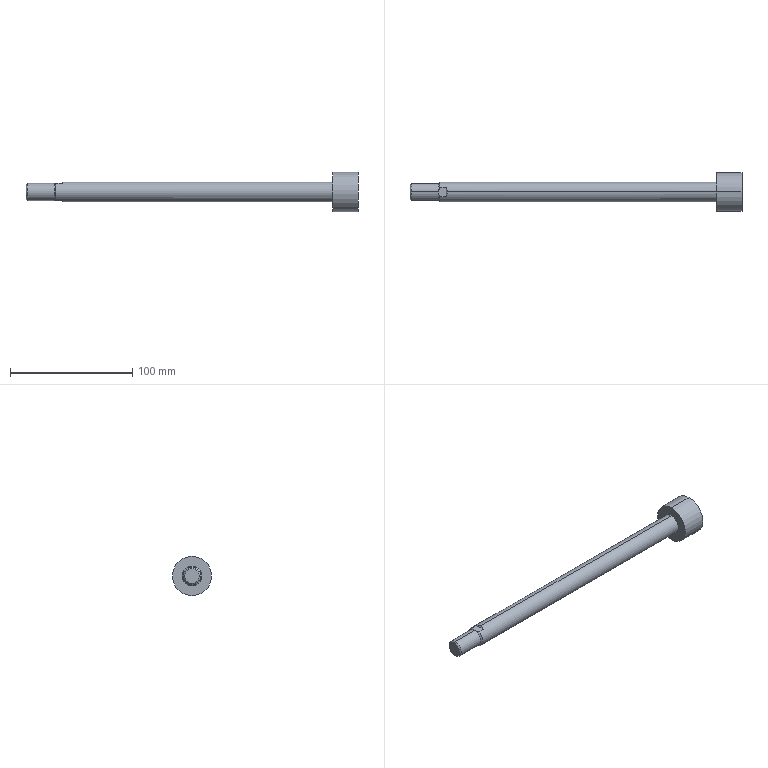Part | STEP file | 1 solid | 17 faces | box 271.5 x 32 x 32 mm | volume 65744 mm3 | plane 7 | cylinder 6 | cone 4 | commonest cylinder face diameters 14 x2 16 x2 32 x2
STEP:
#1=CARTESIAN_POINT('',(0.,0.,0.));
#2=DIRECTION('',(0.,0.,1.));
#3=DIRECTION('',(1.,0.,0.));
#4=AXIS2_PLACEMENT_3D('',#1,#2,#3);
#5=CARTESIAN_POINT('',(-15.,0.,7.));
#6=VERTEX_POINT('',#5);
#7=CARTESIAN_POINT('',(-15.,0.,-7.));
#8=VERTEX_POINT('',#7);
#9=CARTESIAN_POINT('',(-15.,0.,0.));
#10=DIRECTION('',(-1.,0.,0.));
#11=DIRECTION('',(0.,0.,1.));
#12=AXIS2_PLACEMENT_3D('',#9,#10,#11);
#13=CIRCLE('',#12,7.);
#14=CARTESIAN_POINT('',(0.,0.,0.));
#15=DIRECTION('',(-1.,0.,0.));
#16=DIRECTION('',(0.,0.,1.));
#17=AXIS2_PLACEMENT_3D('',#14,#15,#16);
#18=CYLINDRICAL_SURFACE('',#17,7.);
#19=CARTESIAN_POINT('',(0.,15.));
#20=DIRECTION('',(1.,0.));
#21=VECTOR('',#20,1.);
#22=LINE('',#19,#21);
#23=(GEOMETRIC_REPRESENTATION_CONTEXT(2)PARAMETRIC_REPRESENTATION_CONTEXT()REPRESENTATION_CONTEXT('',''));
#24=DEFINITIONAL_REPRESENTATION('',(#22),#23);
#25=PCURVE('',#18,#24);
#26=CARTESIAN_POINT('',(-14.,0.,0.));
#27=DIRECTION('',(1.,0.,0.));
#28=DIRECTION('',(0.,0.,-1.));
#29=AXIS2_PLACEMENT_3D('',#26,#27,#28);
#30=CONICAL_SURFACE('',#29,8.,0.7854);
#31=CARTESIAN_POINT('',(3.142,-1.));
#32=DIRECTION('',(-1.,0.));
#33=VECTOR('',#32,1.);
#34=LINE('',#31,#33);
#35=(GEOMETRIC_REPRESENTATION_CONTEXT(2)PARAMETRIC_REPRESENTATION_CONTEXT()REPRESENTATION_CONTEXT('',''));
#36=DEFINITIONAL_REPRESENTATION('',(#34),#35);
#37=PCURVE('',#30,#36);
#38=SURFACE_CURVE('',#13,(#25,#37),.PCURVE_S1.);
#39=EDGE_CURVE('',#6,#8,#38,.T.);
#40=ORIENTED_EDGE('',*,*,#39,.T.);
#41=CARTESIAN_POINT('',(-37.58,0.,-7.));
#42=VERTEX_POINT('',#41);
#43=CARTESIAN_POINT('',(0.,0.,-7.));
#44=DIRECTION('',(-1.,0.,0.));
#45=VECTOR('',#44,1.);
#46=LINE('',#43,#45);
#47=CARTESIAN_POINT('',(3.142,0.));
#48=DIRECTION('',(0.,1.));
#49=VECTOR('',#48,1.);
#50=LINE('',#47,#49);
#51=(GEOMETRIC_REPRESENTATION_CONTEXT(2)PARAMETRIC_REPRESENTATION_CONTEXT()REPRESENTATION_CONTEXT('',''));
#52=DEFINITIONAL_REPRESENTATION('',(#50),#51);
#53=PCURVE('',#18,#52);
#54=CARTESIAN_POINT('',(0.,0.,0.));
#55=DIRECTION('',(-1.,0.,0.));
#56=DIRECTION('',(0.,0.,1.));
#57=AXIS2_PLACEMENT_3D('',#54,#55,#56);
#58=CYLINDRICAL_SURFACE('',#57,7.);
#59=CARTESIAN_POINT('',(3.142,0.));
#60=DIRECTION('',(0.,1.));
#61=VECTOR('',#60,1.);
#62=LINE('',#59,#61);
#63=(GEOMETRIC_REPRESENTATION_CONTEXT(2)PARAMETRIC_REPRESENTATION_CONTEXT()REPRESENTATION_CONTEXT('',''));
#64=DEFINITIONAL_REPRESENTATION('',(#62),#63);
#65=PCURVE('',#58,#64);
#66=SURFACE_CURVE('',#46,(#53,#65),.PCURVE_S1.);
#67=EDGE_CURVE('',#8,#42,#66,.T.);
#68=ORIENTED_EDGE('',*,*,#67,.T.);
#69=CARTESIAN_POINT('',(-37.58,0.,7.));
#70=VERTEX_POINT('',#69);
#71=CARTESIAN_POINT('',(-37.58,0.,0.));
#72=DIRECTION('',(-1.,0.,0.));
#73=DIRECTION('',(0.,0.,1.));
#74=AXIS2_PLACEMENT_3D('',#71,#72,#73);
#75=CIRCLE('',#74,7.);
#76=CARTESIAN_POINT('',(0.,37.58));
#77=DIRECTION('',(1.,0.));
#78=VECTOR('',#77,1.);
#79=LINE('',#76,#78);
#80=(GEOMETRIC_REPRESENTATION_CONTEXT(2)PARAMETRIC_REPRESENTATION_CONTEXT()REPRESENTATION_CONTEXT('',''));
#81=DEFINITIONAL_REPRESENTATION('',(#79),#80);
#82=PCURVE('',#18,#81);
#83=CARTESIAN_POINT('',(-37.58,0.,0.));
#84=DIRECTION('',(1.,0.,0.));
#85=DIRECTION('',(0.,0.,-1.));
#86=AXIS2_PLACEMENT_3D('',#83,#84,#85);
#87=CONICAL_SURFACE('',#86,7.,0.7854);
#88=CARTESIAN_POINT('',(3.142,0.));
#89=DIRECTION('',(-1.,0.));
#90=VECTOR('',#89,1.);
#91=LINE('',#88,#90);
#92=(GEOMETRIC_REPRESENTATION_CONTEXT(2)PARAMETRIC_REPRESENTATION_CONTEXT()REPRESENTATION_CONTEXT('',''));
#93=DEFINITIONAL_REPRESENTATION('',(#91),#92);
#94=PCURVE('',#87,#93);
#95=SURFACE_CURVE('',#75,(#82,#94),.PCURVE_S1.);
#96=EDGE_CURVE('',#70,#42,#95,.T.);
#97=ORIENTED_EDGE('',*,*,#96,.F.);
#98=CARTESIAN_POINT('',(0.,0.,7.));
#99=DIRECTION('',(-1.,0.,0.));
#100=VECTOR('',#99,1.);
#101=LINE('',#98,#100);
#102=CARTESIAN_POINT('',(0.,0.));
#103=DIRECTION('',(0.,1.));
#104=VECTOR('',#103,1.);
#105=LINE('',#102,#104);
#106=(GEOMETRIC_REPRESENTATION_CONTEXT(2)PARAMETRIC_REPRESENTATION_CONTEXT()REPRESENTATION_CONTEXT('',''));
#107=DEFINITIONAL_REPRESENTATION('',(#105),#106);
#108=PCURVE('',#18,#107);
#109=CARTESIAN_POINT('',(6.283,0.));
#110=DIRECTION('',(0.,1.));
#111=VECTOR('',#110,1.);
#112=LINE('',#109,#111);
#113=(GEOMETRIC_REPRESENTATION_CONTEXT(2)PARAMETRIC_REPRESENTATION_CONTEXT()REPRESENTATION_CONTEXT('',''));
#114=DEFINITIONAL_REPRESENTATION('',(#112),#113);
#115=PCURVE('',#58,#114);
#116=SURFACE_CURVE('',#101,(#108,#115),.PCURVE_S1.);
#117=EDGE_CURVE('',#6,#70,#116,.T.);
#118=ORIENTED_EDGE('',*,*,#117,.F.);
#119=EDGE_LOOP('',(#40,#68,#97,#118));
#120=FACE_BOUND('',#119,.T.);
#121=ADVANCED_FACE('',(#120),#18,.T.);
#122=CARTESIAN_POINT('',(-38.5,0.,6.08));
#123=VERTEX_POINT('',#122);
#124=CARTESIAN_POINT('',(-38.5,0.,-6.08));
#125=VERTEX_POINT('',#124);
#126=CARTESIAN_POINT('',(-38.5,0.,0.));
#127=DIRECTION('',(-1.,0.,0.));
#128=DIRECTION('',(0.,0.,1.));
#129=AXIS2_PLACEMENT_3D('',#126,#127,#128);
#130=CIRCLE('',#129,6.08);
#131=CARTESIAN_POINT('',(3.142,-0.92));
#132=DIRECTION('',(-1.,0.));
#133=VECTOR('',#132,1.);
#134=LINE('',#131,#133);
#135=(GEOMETRIC_REPRESENTATION_CONTEXT(2)PARAMETRIC_REPRESENTATION_CONTEXT()REPRESENTATION_CONTEXT('',''));
#136=DEFINITIONAL_REPRESENTATION('',(#134),#135);
#137=PCURVE('',#87,#136);
#138=CARTESIAN_POINT('',(-38.5,0.,0.));
#139=DIRECTION('',(1.,0.,0.));
#140=DIRECTION('',(0.,0.,-1.));
#141=AXIS2_PLACEMENT_3D('',#138,#139,#140);
#142=PLANE('',#141);
#143=CARTESIAN_POINT('',(-6.08,0.));
#144=CARTESIAN_POINT('',(-6.08,10.531));
#145=CARTESIAN_POINT('',(3.04,5.265));
#146=CARTESIAN_POINT('',(12.16,0.));
#147=CARTESIAN_POINT('',(3.04,-5.265));
#148=CARTESIAN_POINT('',(-6.08,-10.531));
#149=CARTESIAN_POINT('',(-6.08,0.));
#150=(BOUNDED_CURVE()B_SPLINE_CURVE(2,(#143,#144,#145,#146,#147,#148,#149),.UNSPECIFIED.,.T.,.F.)B_SPLINE_CURVE_WITH_KNOTS((1,2,2,2,2,1),(-2.094,0.,2.094,4.189,6.283,8.378),.UNSPECIFIED.)CURVE()GEOMETRIC_REPRESENTATION_ITEM()RATIONAL_B_SPLINE_CURVE((1.,0.5,1.,0.5,1.,0.5,1.))REPRESENTATION_ITEM(''));
#151=(GEOMETRIC_REPRESENTATION_CONTEXT(2)PARAMETRIC_REPRESENTATION_CONTEXT()REPRESENTATION_CONTEXT('',''));
#152=DEFINITIONAL_REPRESENTATION('',(#150),#151);
#153=PCURVE('',#142,#152);
#154=SURFACE_CURVE('',#130,(#137,#153),.PCURVE_S1.);
#155=EDGE_CURVE('',#123,#125,#154,.T.);
#156=ORIENTED_EDGE('',*,*,#155,.F.);
#157=CARTESIAN_POINT('',(-37.58,0.,7.));
#158=DIRECTION('',(0.7071,0.,0.7071));
#159=VECTOR('',#158,1.);
#160=LINE('',#157,#159);
#161=CARTESIAN_POINT('',(3.142,0.));
#162=DIRECTION('',(0.,1.));
#163=VECTOR('',#162,1.);
#164=LINE('',#161,#163);
#165=(GEOMETRIC_REPRESENTATION_CONTEXT(2)PARAMETRIC_REPRESENTATION_CONTEXT()REPRESENTATION_CONTEXT('',''));
#166=DEFINITIONAL_REPRESENTATION('',(#164),#165);
#167=PCURVE('',#87,#166);
#168=CARTESIAN_POINT('',(-37.58,0.,0.));
#169=DIRECTION('',(1.,0.,0.));
#170=DIRECTION('',(0.,0.,-1.));
#171=AXIS2_PLACEMENT_3D('',#168,#169,#170);
#172=CONICAL_SURFACE('',#171,7.,0.7854);
#173=CARTESIAN_POINT('',(3.142,0.));
#174=DIRECTION('',(0.,1.));
#175=VECTOR('',#174,1.);
#176=LINE('',#173,#175);
#177=(GEOMETRIC_REPRESENTATION_CONTEXT(2)PARAMETRIC_REPRESENTATION_CONTEXT()REPRESENTATION_CONTEXT('',''));
#178=DEFINITIONAL_REPRESENTATION('',(#176),#177);
#179=PCURVE('',#172,#178);
#180=SURFACE_CURVE('',#160,(#167,#179),.PCURVE_S1.);
#181=EDGE_CURVE('',#123,#70,#180,.T.);
#182=ORIENTED_EDGE('',*,*,#181,.T.);
#183=ORIENTED_EDGE('',*,*,#96,.T.);
#184=CARTESIAN_POINT('',(-37.58,0.,-7.));
#185=DIRECTION('',(0.7071,0.,-0.7071));
#186=VECTOR('',#185,1.);
#187=LINE('',#184,#186);
#188=CARTESIAN_POINT('',(0.,0.));
#189=DIRECTION('',(0.,1.));
#190=VECTOR('',#189,1.);
#191=LINE('',#188,#190);
#192=(GEOMETRIC_REPRESENTATION_CONTEXT(2)PARAMETRIC_REPRESENTATION_CONTEXT()REPRESENTATION_CONTEXT('',''));
#193=DEFINITIONAL_REPRESENTATION('',(#191),#192);
#194=PCURVE('',#87,#193);
#195=CARTESIAN_POINT('',(6.283,0.));
#196=DIRECTION('',(0.,1.));
#197=VECTOR('',#196,1.);
#198=LINE('',#195,#197);
#199=(GEOMETRIC_REPRESENTATION_CONTEXT(2)PARAMETRIC_REPRESENTATION_CONTEXT()REPRESENTATION_CONTEXT('',''));
#200=DEFINITIONAL_REPRESENTATION('',(#198),#199);
#201=PCURVE('',#172,#200);
#202=SURFACE_CURVE('',#187,(#194,#201),.PCURVE_S1.);
#203=EDGE_CURVE('',#125,#42,#202,.T.);
#204=ORIENTED_EDGE('',*,*,#203,.F.);
#205=EDGE_LOOP('',(#156,#182,#183,#204));
#206=FACE_BOUND('',#205,.T.);
#207=ADVANCED_FACE('',(#206),#87,.T.);
#208=CARTESIAN_POINT('',(233.,0.,16.));
#209=VERTEX_POINT('',#208);
#210=CARTESIAN_POINT('',(233.,0.,-16.));
#211=VERTEX_POINT('',#210);
#212=CARTESIAN_POINT('',(233.,0.,0.));
#213=DIRECTION('',(-1.,0.,0.));
#214=DIRECTION('',(0.,0.,1.));
#215=AXIS2_PLACEMENT_3D('',#212,#213,#214);
#216=CIRCLE('',#215,16.);
#217=CARTESIAN_POINT('',(233.,0.,0.));
#218=DIRECTION('',(-1.,0.,0.));
#219=DIRECTION('',(0.,0.,1.));
#220=AXIS2_PLACEMENT_3D('',#217,#218,#219);
#221=CYLINDRICAL_SURFACE('',#220,16.);
#222=CARTESIAN_POINT('',(0.,0.));
#223=DIRECTION('',(1.,0.));
#224=VECTOR('',#223,1.);
#225=LINE('',#222,#224);
#226=(GEOMETRIC_REPRESENTATION_CONTEXT(2)PARAMETRIC_REPRESENTATION_CONTEXT()REPRESENTATION_CONTEXT('',''));
#227=DEFINITIONAL_REPRESENTATION('',(#225),#226);
#228=PCURVE('',#221,#227);
#229=CARTESIAN_POINT('',(233.,16.,0.));
#230=DIRECTION('',(-1.,0.,0.));
#231=DIRECTION('',(0.,0.,1.));
#232=AXIS2_PLACEMENT_3D('',#229,#230,#231);
#233=PLANE('',#232);
#234=CARTESIAN_POINT('',(0.,-16.));
#235=DIRECTION('',(1.,0.));
#236=AXIS2_PLACEMENT_2D('',#234,#235);
#237=CIRCLE('',#236,16.);
#238=(GEOMETRIC_REPRESENTATION_CONTEXT(2)PARAMETRIC_REPRESENTATION_CONTEXT()REPRESENTATION_CONTEXT('',''));
#239=DEFINITIONAL_REPRESENTATION('',(#237),#238);
#240=PCURVE('',#233,#239);
#241=SURFACE_CURVE('',#216,(#228,#240),.PCURVE_S1.);
#242=EDGE_CURVE('',#209,#211,#241,.T.);
#243=ORIENTED_EDGE('',*,*,#242,.T.);
#244=CARTESIAN_POINT('',(212.5,0.,-16.));
#245=VERTEX_POINT('',#244);
#246=CARTESIAN_POINT('',(233.,0.,-16.));
#247=DIRECTION('',(-1.,0.,0.));
#248=VECTOR('',#247,1.);
#249=LINE('',#246,#248);
#250=CARTESIAN_POINT('',(3.142,0.));
#251=DIRECTION('',(0.,1.));
#252=VECTOR('',#251,1.);
#253=LINE('',#250,#252);
#254=(GEOMETRIC_REPRESENTATION_CONTEXT(2)PARAMETRIC_REPRESENTATION_CONTEXT()REPRESENTATION_CONTEXT('',''));
#255=DEFINITIONAL_REPRESENTATION('',(#253),#254);
#256=PCURVE('',#221,#255);
#257=CARTESIAN_POINT('',(233.,0.,0.));
#258=DIRECTION('',(-1.,0.,0.));
#259=DIRECTION('',(0.,0.,1.));
#260=AXIS2_PLACEMENT_3D('',#257,#258,#259);
#261=CYLINDRICAL_SURFACE('',#260,16.);
#262=CARTESIAN_POINT('',(3.142,0.));
#263=DIRECTION('',(0.,1.));
#264=VECTOR('',#263,1.);
#265=LINE('',#262,#264);
#266=(GEOMETRIC_REPRESENTATION_CONTEXT(2)PARAMETRIC_REPRESENTATION_CONTEXT()REPRESENTATION_CONTEXT('',''));
#267=DEFINITIONAL_REPRESENTATION('',(#265),#266);
#268=PCURVE('',#261,#267);
#269=SURFACE_CURVE('',#249,(#256,#268),.PCURVE_S1.);
#270=EDGE_CURVE('',#211,#245,#269,.T.);
#271=ORIENTED_EDGE('',*,*,#270,.T.);
#272=CARTESIAN_POINT('',(212.5,0.,16.));
#273=VERTEX_POINT('',#272);
#274=CARTESIAN_POINT('',(212.5,0.,0.));
#275=DIRECTION('',(-1.,0.,0.));
#276=DIRECTION('',(0.,0.,1.));
#277=AXIS2_PLACEMENT_3D('',#274,#275,#276);
#278=CIRCLE('',#277,16.);
#279=CARTESIAN_POINT('',(0.,20.5));
#280=DIRECTION('',(1.,0.));
#281=VECTOR('',#280,1.);
#282=LINE('',#279,#281);
#283=(GEOMETRIC_REPRESENTATION_CONTEXT(2)PARAMETRIC_REPRESENTATION_CONTEXT()REPRESENTATION_CONTEXT('',''));
#284=DEFINITIONAL_REPRESENTATION('',(#282),#283);
#285=PCURVE('',#221,#284);
#286=CARTESIAN_POINT('',(212.5,8.,0.));
#287=DIRECTION('',(1.,0.,0.));
#288=DIRECTION('',(0.,0.,-1.));
#289=AXIS2_PLACEMENT_3D('',#286,#287,#288);
#290=PLANE('',#289);
#291=CARTESIAN_POINT('',(-16.,-8.));
#292=CARTESIAN_POINT('',(-16.,19.713));
#293=CARTESIAN_POINT('',(8.,5.856));
#294=CARTESIAN_POINT('',(32.,-8.));
#295=CARTESIAN_POINT('',(8.,-21.856));
#296=CARTESIAN_POINT('',(-16.,-35.713));
#297=CARTESIAN_POINT('',(-16.,-8.));
#298=(BOUNDED_CURVE()B_SPLINE_CURVE(2,(#291,#292,#293,#294,#295,#296,#297),.UNSPECIFIED.,.T.,.F.)B_SPLINE_CURVE_WITH_KNOTS((1,2,2,2,2,1),(-2.094,0.,2.094,4.189,6.283,8.378),.UNSPECIFIED.)CURVE()GEOMETRIC_REPRESENTATION_ITEM()RATIONAL_B_SPLINE_CURVE((1.,0.5,1.,0.5,1.,0.5,1.))REPRESENTATION_ITEM(''));
#299=(GEOMETRIC_REPRESENTATION_CONTEXT(2)PARAMETRIC_REPRESENTATION_CONTEXT()REPRESENTATION_CONTEXT('',''));
#300=DEFINITIONAL_REPRESENTATION('',(#298),#299);
#301=PCURVE('',#290,#300);
#302=SURFACE_CURVE('',#278,(#285,#301),.PCURVE_S1.);
#303=EDGE_CURVE('',#273,#245,#302,.T.);
#304=ORIENTED_EDGE('',*,*,#303,.F.);
#305=CARTESIAN_POINT('',(233.,0.,16.));
#306=DIRECTION('',(-1.,0.,0.));
#307=VECTOR('',#306,1.);
#308=LINE('',#305,#307);
#309=CARTESIAN_POINT('',(0.,0.));
#310=DIRECTION('',(0.,1.));
#311=VECTOR('',#310,1.);
#312=LINE('',#309,#311);
#313=(GEOMETRIC_REPRESENTATION_CONTEXT(2)PARAMETRIC_REPRESENTATION_CONTEXT()REPRESENTATION_CONTEXT('',''));
#314=DEFINITIONAL_REPRESENTATION('',(#312),#313);
#315=PCURVE('',#221,#314);
#316=CARTESIAN_POINT('',(6.283,0.));
#317=DIRECTION('',(0.,1.));
#318=VECTOR('',#317,1.);
#319=LINE('',#316,#318);
#320=(GEOMETRIC_REPRESENTATION_CONTEXT(2)PARAMETRIC_REPRESENTATION_CONTEXT()REPRESENTATION_CONTEXT('',''));
#321=DEFINITIONAL_REPRESENTATION('',(#319),#320);
#322=PCURVE('',#261,#321);
#323=SURFACE_CURVE('',#308,(#315,#322),.PCURVE_S1.);
#324=EDGE_CURVE('',#209,#273,#323,.T.);
#325=ORIENTED_EDGE('',*,*,#324,.F.);
#326=EDGE_LOOP('',(#243,#271,#304,#325));
#327=FACE_BOUND('',#326,.T.);
#328=ADVANCED_FACE('',(#327),#221,.T.);
#329=CARTESIAN_POINT('',(212.5,0.,8.));
#330=VERTEX_POINT('',#329);
#331=CARTESIAN_POINT('',(212.5,0.,-8.));
#332=VERTEX_POINT('',#331);
#333=CARTESIAN_POINT('',(212.5,0.,0.));
#334=DIRECTION('',(-1.,0.,0.));
#335=DIRECTION('',(0.,0.,1.));
#336=AXIS2_PLACEMENT_3D('',#333,#334,#335);
#337=CIRCLE('',#336,8.);
#338=CARTESIAN_POINT('',(233.,0.,0.));
#339=DIRECTION('',(-1.,0.,0.));
#340=DIRECTION('',(0.,0.,1.));
#341=AXIS2_PLACEMENT_3D('',#338,#339,#340);
#342=CYLINDRICAL_SURFACE('',#341,8.);
#343=CARTESIAN_POINT('',(0.,20.5));
#344=DIRECTION('',(1.,0.));
#345=VECTOR('',#344,1.);
#346=LINE('',#343,#345);
#347=(GEOMETRIC_REPRESENTATION_CONTEXT(2)PARAMETRIC_REPRESENTATION_CONTEXT()REPRESENTATION_CONTEXT('',''));
#348=DEFINITIONAL_REPRESENTATION('',(#346),#347);
#349=PCURVE('',#342,#348);
#350=CARTESIAN_POINT('',(-8.,-8.));
#351=CARTESIAN_POINT('',(-8.,5.856));
#352=CARTESIAN_POINT('',(4.,-1.072));
#353=CARTESIAN_POINT('',(16.,-8.));
#354=CARTESIAN_POINT('',(4.,-14.928));
#355=CARTESIAN_POINT('',(-8.,-21.856));
#356=CARTESIAN_POINT('',(-8.,-8.));
#357=(BOUNDED_CURVE()B_SPLINE_CURVE(2,(#350,#351,#352,#353,#354,#355,#356),.UNSPECIFIED.,.T.,.F.)B_SPLINE_CURVE_WITH_KNOTS((1,2,2,2,2,1),(-2.094,0.,2.094,4.189,6.283,8.378),.UNSPECIFIED.)CURVE()GEOMETRIC_REPRESENTATION_ITEM()RATIONAL_B_SPLINE_CURVE((1.,0.5,1.,0.5,1.,0.5,1.))REPRESENTATION_ITEM(''));
#358=(GEOMETRIC_REPRESENTATION_CONTEXT(2)PARAMETRIC_REPRESENTATION_CONTEXT()REPRESENTATION_CONTEXT('',''));
#359=DEFINITIONAL_REPRESENTATION('',(#357),#358);
#360=PCURVE('',#290,#359);
#361=SURFACE_CURVE('',#337,(#349,#360),.PCURVE_S1.);
#362=EDGE_CURVE('',#330,#332,#361,.T.);
#363=ORIENTED_EDGE('',*,*,#362,.T.);
#364=CARTESIAN_POINT('',(-8.,0.,-8.));
#365=VERTEX_POINT('',#364);
#366=CARTESIAN_POINT('',(233.,0.,-8.));
#367=DIRECTION('',(-1.,0.,0.));
#368=VECTOR('',#367,1.);
#369=LINE('',#366,#368);
#370=CARTESIAN_POINT('',(3.142,0.));
#371=DIRECTION('',(0.,1.));
#372=VECTOR('',#371,1.);
#373=LINE('',#370,#372);
#374=(GEOMETRIC_REPRESENTATION_CONTEXT(2)PARAMETRIC_REPRESENTATION_CONTEXT()REPRESENTATION_CONTEXT('',''));
#375=DEFINITIONAL_REPRESENTATION('',(#373),#374);
#376=PCURVE('',#342,#375);
#377=CARTESIAN_POINT('',(233.,0.,0.));
#378=DIRECTION('',(-1.,0.,0.));
#379=DIRECTION('',(0.,0.,1.));
#380=AXIS2_PLACEMENT_3D('',#377,#378,#379);
#381=CYLINDRICAL_SURFACE('',#380,8.);
#382=CARTESIAN_POINT('',(3.142,0.));
#383=DIRECTION('',(0.,1.));
#384=VECTOR('',#383,1.);
#385=LINE('',#382,#384);
#386=(GEOMETRIC_REPRESENTATION_CONTEXT(2)PARAMETRIC_REPRESENTATION_CONTEXT()REPRESENTATION_CONTEXT('',''));
#387=DEFINITIONAL_REPRESENTATION('',(#385),#386);
#388=PCURVE('',#381,#387);
#389=SURFACE_CURVE('',#369,(#376,#388),.PCURVE_S1.);
#390=EDGE_CURVE('',#332,#365,#389,.T.);
#391=ORIENTED_EDGE('',*,*,#390,.T.);
#392=CARTESIAN_POINT('',(-9.,3.873,-7.));
#393=VERTEX_POINT('',#392);
#394=CARTESIAN_POINT('',(-9.,3.873,-7.));
#395=CARTESIAN_POINT('',(-8.341,2.681,-7.659));
#396=CARTESIAN_POINT('',(-8.,1.362,-8.));
#397=CARTESIAN_POINT('',(-8.,0.,-8.));
#398=(BOUNDED_CURVE()B_SPLINE_CURVE(3,(#394,#395,#396,#397),.UNSPECIFIED.,.F.,.F.)B_SPLINE_CURVE_WITH_KNOTS((4,4),(2.636,3.142),.PIECEWISE_BEZIER_KNOTS.)CURVE()GEOMETRIC_REPRESENTATION_ITEM()RATIONAL_B_SPLINE_CURVE((1.,0.9788,0.9788,1.))REPRESENTATION_ITEM(''));
#399=CARTESIAN_POINT('',(2.636,242.));
#400=CARTESIAN_POINT('',(2.644,241.971));
#401=CARTESIAN_POINT('',(2.659,241.913));
#402=CARTESIAN_POINT('',(2.682,241.83));
#403=CARTESIAN_POINT('',(2.705,241.751));
#404=CARTESIAN_POINT('',(2.728,241.675));
#405=CARTESIAN_POINT('',(2.751,241.603));
#406=CARTESIAN_POINT('',(2.774,241.535));
#407=CARTESIAN_POINT('',(2.797,241.471));
#408=CARTESIAN_POINT('',(2.82,241.41));
#409=CARTESIAN_POINT('',(2.843,241.354));
#410=CARTESIAN_POINT('',(2.866,241.302));
#411=CARTESIAN_POINT('',(2.889,241.253));
#412=CARTESIAN_POINT('',(2.912,241.209));
#413=CARTESIAN_POINT('',(2.935,241.169));
#414=CARTESIAN_POINT('',(2.958,241.134));
#415=CARTESIAN_POINT('',(2.981,241.102));
#416=CARTESIAN_POINT('',(3.004,241.075));
#417=CARTESIAN_POINT('',(3.027,241.052));
#418=CARTESIAN_POINT('',(3.05,241.033));
#419=CARTESIAN_POINT('',(3.073,241.018));
#420=CARTESIAN_POINT('',(3.096,241.008));
#421=CARTESIAN_POINT('',(3.119,241.001));
#422=CARTESIAN_POINT('',(3.134,241.));
#423=CARTESIAN_POINT('',(3.142,241.));
#424=B_SPLINE_CURVE_WITH_KNOTS('',3,(#399,#400,#401,#402,#403,#404,#405,#406,#407,#408,#409,#410,#411,#412,#413,#414,#415,#416,#417,#418,#419,#420,#421,#422,#423),.UNSPECIFIED.,.F.,.F.,(4,1,1,1,1,1,1,1,1,1,1,1,1,1,1,1,1,1,1,1,1,1,4),(2.636,2.659,2.682,2.705,2.728,2.751,2.774,2.797,2.82,2.843,2.866,2.889,2.912,2.935,2.958,2.981,3.004,3.027,3.05,3.073,3.096,3.119,3.142),.QUASI_UNIFORM_KNOTS.);
#425=(GEOMETRIC_REPRESENTATION_CONTEXT(2)PARAMETRIC_REPRESENTATION_CONTEXT()REPRESENTATION_CONTEXT('',''));
#426=DEFINITIONAL_REPRESENTATION('',(#424),#425);
#427=PCURVE('',#342,#426);
#428=CARTESIAN_POINT('',(-9.,32.,-7.));
#429=DIRECTION('',(-0.7071,0.,-0.7071));
#430=DIRECTION('',(-0.7071,0.,0.7071));
#431=AXIS2_PLACEMENT_3D('',#428,#429,#430);
#432=PLANE('',#431);
#433=CARTESIAN_POINT('',(0.,-28.127));
#434=CARTESIAN_POINT('',(-0.9326,-29.319));
#435=CARTESIAN_POINT('',(-1.414,-30.638));
#436=CARTESIAN_POINT('',(-1.414,-32.));
#437=(BOUNDED_CURVE()B_SPLINE_CURVE(3,(#433,#434,#435,#436),.UNSPECIFIED.,.F.,.F.)B_SPLINE_CURVE_WITH_KNOTS((4,4),(2.636,3.142),.PIECEWISE_BEZIER_KNOTS.)CURVE()GEOMETRIC_REPRESENTATION_ITEM()RATIONAL_B_SPLINE_CURVE((1.,0.9788,0.9788,1.))REPRESENTATION_ITEM(''));
#438=(GEOMETRIC_REPRESENTATION_CONTEXT(2)PARAMETRIC_REPRESENTATION_CONTEXT()REPRESENTATION_CONTEXT('',''));
#439=DEFINITIONAL_REPRESENTATION('',(#437),#438);
#440=PCURVE('',#432,#439);
#441=SURFACE_CURVE('',#398,(#427,#440),.PCURVE_S1.);
#442=EDGE_CURVE('',#393,#365,#441,.T.);
#443=ORIENTED_EDGE('',*,*,#442,.F.);
#444=CARTESIAN_POINT('',(-14.,3.873,-7.));
#445=VERTEX_POINT('',#444);
#446=CARTESIAN_POINT('',(233.,3.873,-7.));
#447=DIRECTION('',(1.,0.,0.));
#448=VECTOR('',#447,1.);
#449=LINE('',#446,#448);
#450=CARTESIAN_POINT('',(2.636,0.));
#451=DIRECTION('',(0.,-1.));
#452=VECTOR('',#451,1.);
#453=LINE('',#450,#452);
#454=(GEOMETRIC_REPRESENTATION_CONTEXT(2)PARAMETRIC_REPRESENTATION_CONTEXT()REPRESENTATION_CONTEXT('',''));
#455=DEFINITIONAL_REPRESENTATION('',(#453),#454);
#456=PCURVE('',#342,#455);
#457=CARTESIAN_POINT('',(-15.,32.,-7.));
#458=DIRECTION('',(0.,0.,-1.));
#459=DIRECTION('',(-1.,0.,0.));
#460=AXIS2_PLACEMENT_3D('',#457,#458,#459);
#461=PLANE('',#460);
#462=CARTESIAN_POINT('',(-248.,-28.127));
#463=DIRECTION('',(-1.,0.));
#464=VECTOR('',#463,1.);
#465=LINE('',#462,#464);
#466=(GEOMETRIC_REPRESENTATION_CONTEXT(2)PARAMETRIC_REPRESENTATION_CONTEXT()REPRESENTATION_CONTEXT('',''));
#467=DEFINITIONAL_REPRESENTATION('',(#465),#466);
#468=PCURVE('',#461,#467);
#469=SURFACE_CURVE('',#449,(#456,#468),.PCURVE_S1.);
#470=EDGE_CURVE('',#445,#393,#469,.T.);
#471=ORIENTED_EDGE('',*,*,#470,.F.);
#472=CARTESIAN_POINT('',(-14.,3.873,7.));
#473=VERTEX_POINT('',#472);
#474=CARTESIAN_POINT('',(-14.,0.,0.));
#475=DIRECTION('',(-1.,0.,0.));
#476=DIRECTION('',(0.,0.,1.));
#477=AXIS2_PLACEMENT_3D('',#474,#475,#476);
#478=CIRCLE('',#477,8.);
#479=CARTESIAN_POINT('',(0.,247.));
#480=DIRECTION('',(1.,0.));
#481=VECTOR('',#480,1.);
#482=LINE('',#479,#481);
#483=(GEOMETRIC_REPRESENTATION_CONTEXT(2)PARAMETRIC_REPRESENTATION_CONTEXT()REPRESENTATION_CONTEXT('',''));
#484=DEFINITIONAL_REPRESENTATION('',(#482),#483);
#485=PCURVE('',#342,#484);
#486=CARTESIAN_POINT('',(3.142,0.));
#487=DIRECTION('',(-1.,0.));
#488=VECTOR('',#487,1.);
#489=LINE('',#486,#488);
#490=(GEOMETRIC_REPRESENTATION_CONTEXT(2)PARAMETRIC_REPRESENTATION_CONTEXT()REPRESENTATION_CONTEXT('',''));
#491=DEFINITIONAL_REPRESENTATION('',(#489),#490);
#492=PCURVE('',#30,#491);
#493=SURFACE_CURVE('',#478,(#485,#492),.PCURVE_S1.);
#494=EDGE_CURVE('',#473,#445,#493,.T.);
#495=ORIENTED_EDGE('',*,*,#494,.F.);
#496=CARTESIAN_POINT('',(-9.,3.873,7.));
#497=VERTEX_POINT('',#496);
#498=CARTESIAN_POINT('',(233.,3.873,7.));
#499=DIRECTION('',(-1.,0.,0.));
#500=VECTOR('',#499,1.);
#501=LINE('',#498,#500);
#502=CARTESIAN_POINT('',(0.5054,0.));
#503=DIRECTION('',(0.,1.));
#504=VECTOR('',#503,1.);
#505=LINE('',#502,#504);
#506=(GEOMETRIC_REPRESENTATION_CONTEXT(2)PARAMETRIC_REPRESENTATION_CONTEXT()REPRESENTATION_CONTEXT('',''));
#507=DEFINITIONAL_REPRESENTATION('',(#505),#506);
#508=PCURVE('',#342,#507);
#509=CARTESIAN_POINT('',(-9.,32.,7.));
#510=DIRECTION('',(0.,0.,1.));
#511=DIRECTION('',(1.,0.,0.));
#512=AXIS2_PLACEMENT_3D('',#509,#510,#511);
#513=PLANE('',#512);
#514=CARTESIAN_POINT('',(242.,-28.127));
#515=DIRECTION('',(-1.,0.));
#516=VECTOR('',#515,1.);
#517=LINE('',#514,#516);
#518=(GEOMETRIC_REPRESENTATION_CONTEXT(2)PARAMETRIC_REPRESENTATION_CONTEXT()REPRESENTATION_CONTEXT('',''));
#519=DEFINITIONAL_REPRESENTATION('',(#517),#518);
#520=PCURVE('',#513,#519);
#521=SURFACE_CURVE('',#501,(#508,#520),.PCURVE_S1.);
#522=EDGE_CURVE('',#497,#473,#521,.T.);
#523=ORIENTED_EDGE('',*,*,#522,.F.);
#524=CARTESIAN_POINT('',(-8.,0.,8.));
#525=VERTEX_POINT('',#524);
#526=CARTESIAN_POINT('',(-8.,0.,8.));
#527=CARTESIAN_POINT('',(-8.,1.362,8.));
#528=CARTESIAN_POINT('',(-8.341,2.681,7.659));
#529=CARTESIAN_POINT('',(-9.,3.873,7.));
#530=(BOUNDED_CURVE()B_SPLINE_CURVE(3,(#526,#527,#528,#529),.UNSPECIFIED.,.F.,.F.)B_SPLINE_CURVE_WITH_KNOTS((4,4),(3.142,3.647),.PIECEWISE_BEZIER_KNOTS.)CURVE()GEOMETRIC_REPRESENTATION_ITEM()RATIONAL_B_SPLINE_CURVE((1.,0.9788,0.9788,1.))REPRESENTATION_ITEM(''));
#531=CARTESIAN_POINT('',(0.,241.));
#532=CARTESIAN_POINT('',(0.007576,241.));
#533=CARTESIAN_POINT('',(0.02275,241.001));
#534=CARTESIAN_POINT('',(0.04557,241.008));
#535=CARTESIAN_POINT('',(0.06844,241.018));
#536=CARTESIAN_POINT('',(0.09137,241.033));
#537=CARTESIAN_POINT('',(0.1143,241.052));
#538=CARTESIAN_POINT('',(0.1373,241.075));
#539=CARTESIAN_POINT('',(0.1604,241.102));
#540=CARTESIAN_POINT('',(0.1834,241.134));
#541=CARTESIAN_POINT('',(0.2065,241.169));
#542=CARTESIAN_POINT('',(0.2296,241.209));
#543=CARTESIAN_POINT('',(0.2527,241.253));
#544=CARTESIAN_POINT('',(0.2758,241.302));
#545=CARTESIAN_POINT('',(0.2989,241.354));
#546=CARTESIAN_POINT('',(0.3219,241.41));
#547=CARTESIAN_POINT('',(0.345,241.471));
#548=CARTESIAN_POINT('',(0.368,241.535));
#549=CARTESIAN_POINT('',(0.391,241.603));
#550=CARTESIAN_POINT('',(0.414,241.675));
#551=CARTESIAN_POINT('',(0.4369,241.751));
#552=CARTESIAN_POINT('',(0.4598,241.83));
#553=CARTESIAN_POINT('',(0.4826,241.913));
#554=CARTESIAN_POINT('',(0.4978,241.971));
#555=CARTESIAN_POINT('',(0.5054,242.));
#556=B_SPLINE_CURVE_WITH_KNOTS('',3,(#531,#532,#533,#534,#535,#536,#537,#538,#539,#540,#541,#542,#543,#544,#545,#546,#547,#548,#549,#550,#551,#552,#553,#554,#555),.UNSPECIFIED.,.F.,.F.,(4,1,1,1,1,1,1,1,1,1,1,1,1,1,1,1,1,1,1,1,1,1,4),(3.142,3.165,3.188,3.211,3.233,3.256,3.279,3.302,3.325,3.348,3.371,3.394,3.417,3.44,3.463,3.486,3.509,3.532,3.555,3.578,3.601,3.624,3.647),.QUASI_UNIFORM_KNOTS.);
#557=(GEOMETRIC_REPRESENTATION_CONTEXT(2)PARAMETRIC_REPRESENTATION_CONTEXT()REPRESENTATION_CONTEXT('',''));
#558=DEFINITIONAL_REPRESENTATION('',(#556),#557);
#559=PCURVE('',#342,#558);
#560=CARTESIAN_POINT('',(19.284,32.,35.284));
#561=DIRECTION('',(-0.7071,0.,0.7071));
#562=DIRECTION('',(0.7071,0.,0.7071));
#563=AXIS2_PLACEMENT_3D('',#560,#561,#562);
#564=PLANE('',#563);
#565=CARTESIAN_POINT('',(-38.586,-32.));
#566=CARTESIAN_POINT('',(-38.586,-30.638));
#567=CARTESIAN_POINT('',(-39.067,-29.319));
#568=CARTESIAN_POINT('',(-40.,-28.127));
#569=(BOUNDED_CURVE()B_SPLINE_CURVE(3,(#565,#566,#567,#568),.UNSPECIFIED.,.F.,.F.)B_SPLINE_CURVE_WITH_KNOTS((4,4),(3.142,3.647),.PIECEWISE_BEZIER_KNOTS.)CURVE()GEOMETRIC_REPRESENTATION_ITEM()RATIONAL_B_SPLINE_CURVE((1.,0.9788,0.9788,1.))REPRESENTATION_ITEM(''));
#570=(GEOMETRIC_REPRESENTATION_CONTEXT(2)PARAMETRIC_REPRESENTATION_CONTEXT()REPRESENTATION_CONTEXT('',''));
#571=DEFINITIONAL_REPRESENTATION('',(#569),#570);
#572=PCURVE('',#564,#571);
#573=SURFACE_CURVE('',#530,(#559,#572),.PCURVE_S1.);
#574=EDGE_CURVE('',#525,#497,#573,.T.);
#575=ORIENTED_EDGE('',*,*,#574,.F.);
#576=CARTESIAN_POINT('',(233.,0.,8.));
#577=DIRECTION('',(-1.,0.,0.));
#578=VECTOR('',#577,1.);
#579=LINE('',#576,#578);
#580=CARTESIAN_POINT('',(0.,0.));
#581=DIRECTION('',(0.,1.));
#582=VECTOR('',#581,1.);
#583=LINE('',#580,#582);
#584=(GEOMETRIC_REPRESENTATION_CONTEXT(2)PARAMETRIC_REPRESENTATION_CONTEXT()REPRESENTATION_CONTEXT('',''));
#585=DEFINITIONAL_REPRESENTATION('',(#583),#584);
#586=PCURVE('',#342,#585);
#587=CARTESIAN_POINT('',(6.283,0.));
#588=DIRECTION('',(0.,1.));
#589=VECTOR('',#588,1.);
#590=LINE('',#587,#589);
#591=(GEOMETRIC_REPRESENTATION_CONTEXT(2)PARAMETRIC_REPRESENTATION_CONTEXT()REPRESENTATION_CONTEXT('',''));
#592=DEFINITIONAL_REPRESENTATION('',(#590),#591);
#593=PCURVE('',#381,#592);
#594=SURFACE_CURVE('',#579,(#586,#593),.PCURVE_S1.);
#595=EDGE_CURVE('',#330,#525,#594,.T.);
#596=ORIENTED_EDGE('',*,*,#595,.F.);
#597=EDGE_LOOP('',(#363,#391,#443,#471,#495,#523,#575,#596));
#598=FACE_BOUND('',#597,.T.);
#599=ADVANCED_FACE('',(#598),#342,.T.);
#600=ORIENTED_EDGE('',*,*,#390,.F.);
#601=CARTESIAN_POINT('',(212.5,0.,0.));
#602=DIRECTION('',(-1.,0.,0.));
#603=DIRECTION('',(0.,0.,1.));
#604=AXIS2_PLACEMENT_3D('',#601,#602,#603);
#605=CIRCLE('',#604,8.);
#606=CARTESIAN_POINT('',(0.,20.5));
#607=DIRECTION('',(1.,0.));
#608=VECTOR('',#607,1.);
#609=LINE('',#606,#608);
#610=(GEOMETRIC_REPRESENTATION_CONTEXT(2)PARAMETRIC_REPRESENTATION_CONTEXT()REPRESENTATION_CONTEXT('',''));
#611=DEFINITIONAL_REPRESENTATION('',(#609),#610);
#612=PCURVE('',#381,#611);
#613=CARTESIAN_POINT('',(-8.,-8.));
#614=CARTESIAN_POINT('',(-8.,5.856));
#615=CARTESIAN_POINT('',(4.,-1.072));
#616=CARTESIAN_POINT('',(16.,-8.));
#617=CARTESIAN_POINT('',(4.,-14.928));
#618=CARTESIAN_POINT('',(-8.,-21.856));
#619=CARTESIAN_POINT('',(-8.,-8.));
#620=(BOUNDED_CURVE()B_SPLINE_CURVE(2,(#613,#614,#615,#616,#617,#618,#619),.UNSPECIFIED.,.T.,.F.)B_SPLINE_CURVE_WITH_KNOTS((1,2,2,2,2,1),(-2.094,0.,2.094,4.189,6.283,8.378),.UNSPECIFIED.)CURVE()GEOMETRIC_REPRESENTATION_ITEM()RATIONAL_B_SPLINE_CURVE((1.,0.5,1.,0.5,1.,0.5,1.))REPRESENTATION_ITEM(''));
#621=(GEOMETRIC_REPRESENTATION_CONTEXT(2)PARAMETRIC_REPRESENTATION_CONTEXT()REPRESENTATION_CONTEXT('',''));
#622=DEFINITIONAL_REPRESENTATION('',(#620),#621);
#623=PCURVE('',#290,#622);
#624=SURFACE_CURVE('',#605,(#612,#623),.PCURVE_S1.);
#625=EDGE_CURVE('',#332,#330,#624,.T.);
#626=ORIENTED_EDGE('',*,*,#625,.T.);
#627=ORIENTED_EDGE('',*,*,#595,.T.);
#628=CARTESIAN_POINT('',(-9.,-3.873,7.));
#629=VERTEX_POINT('',#628);
#630=CARTESIAN_POINT('',(-9.,-3.873,7.));
#631=CARTESIAN_POINT('',(-8.341,-2.681,7.659));
#632=CARTESIAN_POINT('',(-8.,-1.362,8.));
#633=CARTESIAN_POINT('',(-8.,0.,8.));
#634=(BOUNDED_CURVE()B_SPLINE_CURVE(3,(#630,#631,#632,#633),.UNSPECIFIED.,.F.,.F.)B_SPLINE_CURVE_WITH_KNOTS((4,4),(2.636,3.142),.PIECEWISE_BEZIER_KNOTS.)CURVE()GEOMETRIC_REPRESENTATION_ITEM()RATIONAL_B_SPLINE_CURVE((1.,0.9788,0.9788,1.))REPRESENTATION_ITEM(''));
#635=CARTESIAN_POINT('',(5.778,242.));
#636=CARTESIAN_POINT('',(5.785,241.971));
#637=CARTESIAN_POINT('',(5.801,241.913));
#638=CARTESIAN_POINT('',(5.823,241.83));
#639=CARTESIAN_POINT('',(5.846,241.751));
#640=CARTESIAN_POINT('',(5.869,241.675));
#641=CARTESIAN_POINT('',(5.892,241.603));
#642=CARTESIAN_POINT('',(5.915,241.535));
#643=CARTESIAN_POINT('',(5.938,241.471));
#644=CARTESIAN_POINT('',(5.961,241.41));
#645=CARTESIAN_POINT('',(5.984,241.354));
#646=CARTESIAN_POINT('',(6.007,241.302));
#647=CARTESIAN_POINT('',(6.031,241.253));
#648=CARTESIAN_POINT('',(6.054,241.209));
#649=CARTESIAN_POINT('',(6.077,241.169));
#650=CARTESIAN_POINT('',(6.1,241.134));
#651=CARTESIAN_POINT('',(6.123,241.102));
#652=CARTESIAN_POINT('',(6.146,241.075));
#653=CARTESIAN_POINT('',(6.169,241.052));
#654=CARTESIAN_POINT('',(6.192,241.033));
#655=CARTESIAN_POINT('',(6.215,241.018));
#656=CARTESIAN_POINT('',(6.238,241.008));
#657=CARTESIAN_POINT('',(6.26,241.001));
#658=CARTESIAN_POINT('',(6.276,241.));
#659=CARTESIAN_POINT('',(6.283,241.));
#660=B_SPLINE_CURVE_WITH_KNOTS('',3,(#635,#636,#637,#638,#639,#640,#641,#642,#643,#644,#645,#646,#647,#648,#649,#650,#651,#652,#653,#654,#655,#656,#657,#658,#659),.UNSPECIFIED.,.F.,.F.,(4,1,1,1,1,1,1,1,1,1,1,1,1,1,1,1,1,1,1,1,1,1,4),(2.636,2.659,2.682,2.705,2.728,2.751,2.774,2.797,2.82,2.843,2.866,2.889,2.912,2.935,2.958,2.981,3.004,3.027,3.05,3.073,3.096,3.119,3.142),.QUASI_UNIFORM_KNOTS.);
#661=(GEOMETRIC_REPRESENTATION_CONTEXT(2)PARAMETRIC_REPRESENTATION_CONTEXT()REPRESENTATION_CONTEXT('',''));
#662=DEFINITIONAL_REPRESENTATION('',(#660),#661);
#663=PCURVE('',#381,#662);
#664=CARTESIAN_POINT('',(-40.,-35.873));
#665=CARTESIAN_POINT('',(-39.067,-34.681));
#666=CARTESIAN_POINT('',(-38.586,-33.362));
#667=CARTESIAN_POINT('',(-38.586,-32.));
#668=(BOUNDED_CURVE()B_SPLINE_CURVE(3,(#664,#665,#666,#667),.UNSPECIFIED.,.F.,.F.)B_SPLINE_CURVE_WITH_KNOTS((4,4),(2.636,3.142),.PIECEWISE_BEZIER_KNOTS.)CURVE()GEOMETRIC_REPRESENTATION_ITEM()RATIONAL_B_SPLINE_CURVE((1.,0.9788,0.9788,1.))REPRESENTATION_ITEM(''));
#669=(GEOMETRIC_REPRESENTATION_CONTEXT(2)PARAMETRIC_REPRESENTATION_CONTEXT()REPRESENTATION_CONTEXT('',''));
#670=DEFINITIONAL_REPRESENTATION('',(#668),#669);
#671=PCURVE('',#564,#670);
#672=SURFACE_CURVE('',#634,(#663,#671),.PCURVE_S1.);
#673=EDGE_CURVE('',#629,#525,#672,.T.);
#674=ORIENTED_EDGE('',*,*,#673,.F.);
#675=CARTESIAN_POINT('',(-14.,-3.873,7.));
#676=VERTEX_POINT('',#675);
#677=CARTESIAN_POINT('',(233.,-3.873,7.));
#678=DIRECTION('',(1.,0.,0.));
#679=VECTOR('',#678,1.);
#680=LINE('',#677,#679);
#681=CARTESIAN_POINT('',(5.778,0.));
#682=DIRECTION('',(0.,-1.));
#683=VECTOR('',#682,1.);
#684=LINE('',#681,#683);
#685=(GEOMETRIC_REPRESENTATION_CONTEXT(2)PARAMETRIC_REPRESENTATION_CONTEXT()REPRESENTATION_CONTEXT('',''));
#686=DEFINITIONAL_REPRESENTATION('',(#684),#685);
#687=PCURVE('',#381,#686);
#688=CARTESIAN_POINT('',(242.,-35.873));
#689=DIRECTION('',(1.,0.));
#690=VECTOR('',#689,1.);
#691=LINE('',#688,#690);
#692=(GEOMETRIC_REPRESENTATION_CONTEXT(2)PARAMETRIC_REPRESENTATION_CONTEXT()REPRESENTATION_CONTEXT('',''));
#693=DEFINITIONAL_REPRESENTATION('',(#691),#692);
#694=PCURVE('',#513,#693);
#695=SURFACE_CURVE('',#680,(#687,#694),.PCURVE_S1.);
#696=EDGE_CURVE('',#676,#629,#695,.T.);
#697=ORIENTED_EDGE('',*,*,#696,.F.);
#698=CARTESIAN_POINT('',(-14.,-3.873,-7.));
#699=VERTEX_POINT('',#698);
#700=CARTESIAN_POINT('',(-14.,0.,0.));
#701=DIRECTION('',(-1.,0.,0.));
#702=DIRECTION('',(0.,0.,1.));
#703=AXIS2_PLACEMENT_3D('',#700,#701,#702);
#704=CIRCLE('',#703,8.);
#705=CARTESIAN_POINT('',(0.,247.));
#706=DIRECTION('',(1.,0.));
#707=VECTOR('',#706,1.);
#708=LINE('',#705,#707);
#709=(GEOMETRIC_REPRESENTATION_CONTEXT(2)PARAMETRIC_REPRESENTATION_CONTEXT()REPRESENTATION_CONTEXT('',''));
#710=DEFINITIONAL_REPRESENTATION('',(#708),#709);
#711=PCURVE('',#381,#710);
#712=CARTESIAN_POINT('',(-14.,0.,0.));
#713=DIRECTION('',(1.,0.,0.));
#714=DIRECTION('',(0.,0.,-1.));
#715=AXIS2_PLACEMENT_3D('',#712,#713,#714);
#716=CONICAL_SURFACE('',#715,8.,0.7854);
#717=CARTESIAN_POINT('',(9.425,0.));
#718=DIRECTION('',(-1.,0.));
#719=VECTOR('',#718,1.);
#720=LINE('',#717,#719);
#721=(GEOMETRIC_REPRESENTATION_CONTEXT(2)PARAMETRIC_REPRESENTATION_CONTEXT()REPRESENTATION_CONTEXT('',''));
#722=DEFINITIONAL_REPRESENTATION('',(#720),#721);
#723=PCURVE('',#716,#722);
#724=SURFACE_CURVE('',#704,(#711,#723),.PCURVE_S1.);
#725=EDGE_CURVE('',#699,#676,#724,.T.);
#726=ORIENTED_EDGE('',*,*,#725,.F.);
#727=CARTESIAN_POINT('',(-9.,-3.873,-7.));
#728=VERTEX_POINT('',#727);
#729=CARTESIAN_POINT('',(233.,-3.873,-7.));
#730=DIRECTION('',(-1.,0.,0.));
#731=VECTOR('',#730,1.);
#732=LINE('',#729,#731);
#733=CARTESIAN_POINT('',(3.647,0.));
#734=DIRECTION('',(0.,1.));
#735=VECTOR('',#734,1.);
#736=LINE('',#733,#735);
#737=(GEOMETRIC_REPRESENTATION_CONTEXT(2)PARAMETRIC_REPRESENTATION_CONTEXT()REPRESENTATION_CONTEXT('',''));
#738=DEFINITIONAL_REPRESENTATION('',(#736),#737);
#739=PCURVE('',#381,#738);
#740=CARTESIAN_POINT('',(-248.,-35.873));
#741=DIRECTION('',(1.,0.));
#742=VECTOR('',#741,1.);
#743=LINE('',#740,#742);
#744=(GEOMETRIC_REPRESENTATION_CONTEXT(2)PARAMETRIC_REPRESENTATION_CONTEXT()REPRESENTATION_CONTEXT('',''));
#745=DEFINITIONAL_REPRESENTATION('',(#743),#744);
#746=PCURVE('',#461,#745);
#747=SURFACE_CURVE('',#732,(#739,#746),.PCURVE_S1.);
#748=EDGE_CURVE('',#728,#699,#747,.T.);
#749=ORIENTED_EDGE('',*,*,#748,.F.);
#750=CARTESIAN_POINT('',(-8.,0.,-8.));
#751=CARTESIAN_POINT('',(-8.,-1.362,-8.));
#752=CARTESIAN_POINT('',(-8.341,-2.681,-7.659));
#753=CARTESIAN_POINT('',(-9.,-3.873,-7.));
#754=(BOUNDED_CURVE()B_SPLINE_CURVE(3,(#750,#751,#752,#753),.UNSPECIFIED.,.F.,.F.)B_SPLINE_CURVE_WITH_KNOTS((4,4),(3.142,3.647),.PIECEWISE_BEZIER_KNOTS.)CURVE()GEOMETRIC_REPRESENTATION_ITEM()RATIONAL_B_SPLINE_CURVE((1.,0.9788,0.9788,1.))REPRESENTATION_ITEM(''));
#755=CARTESIAN_POINT('',(3.142,241.));
#756=CARTESIAN_POINT('',(3.149,241.));
#757=CARTESIAN_POINT('',(3.164,241.001));
#758=CARTESIAN_POINT('',(3.187,241.008));
#759=CARTESIAN_POINT('',(3.21,241.018));
#760=CARTESIAN_POINT('',(3.233,241.033));
#761=CARTESIAN_POINT('',(3.256,241.052));
#762=CARTESIAN_POINT('',(3.279,241.075));
#763=CARTESIAN_POINT('',(3.302,241.102));
#764=CARTESIAN_POINT('',(3.325,241.134));
#765=CARTESIAN_POINT('',(3.348,241.169));
#766=CARTESIAN_POINT('',(3.371,241.209));
#767=CARTESIAN_POINT('',(3.394,241.253));
#768=CARTESIAN_POINT('',(3.417,241.302));
#769=CARTESIAN_POINT('',(3.44,241.354));
#770=CARTESIAN_POINT('',(3.464,241.41));
#771=CARTESIAN_POINT('',(3.487,241.471));
#772=CARTESIAN_POINT('',(3.51,241.535));
#773=CARTESIAN_POINT('',(3.533,241.603));
#774=CARTESIAN_POINT('',(3.556,241.675));
#775=CARTESIAN_POINT('',(3.579,241.751));
#776=CARTESIAN_POINT('',(3.601,241.83));
#777=CARTESIAN_POINT('',(3.624,241.913));
#778=CARTESIAN_POINT('',(3.639,241.971));
#779=CARTESIAN_POINT('',(3.647,242.));
#780=B_SPLINE_CURVE_WITH_KNOTS('',3,(#755,#756,#757,#758,#759,#760,#761,#762,#763,#764,#765,#766,#767,#768,#769,#770,#771,#772,#773,#774,#775,#776,#777,#778,#779),.UNSPECIFIED.,.F.,.F.,(4,1,1,1,1,1,1,1,1,1,1,1,1,1,1,1,1,1,1,1,1,1,4),(3.142,3.165,3.188,3.211,3.233,3.256,3.279,3.302,3.325,3.348,3.371,3.394,3.417,3.44,3.463,3.486,3.509,3.532,3.555,3.578,3.601,3.624,3.647),.QUASI_UNIFORM_KNOTS.);
#781=(GEOMETRIC_REPRESENTATION_CONTEXT(2)PARAMETRIC_REPRESENTATION_CONTEXT()REPRESENTATION_CONTEXT('',''));
#782=DEFINITIONAL_REPRESENTATION('',(#780),#781);
#783=PCURVE('',#381,#782);
#784=CARTESIAN_POINT('',(-1.414,-32.));
#785=CARTESIAN_POINT('',(-1.414,-33.362));
#786=CARTESIAN_POINT('',(-0.9326,-34.681));
#787=CARTESIAN_POINT('',(0.,-35.873));
#788=(BOUNDED_CURVE()B_SPLINE_CURVE(3,(#784,#785,#786,#787),.UNSPECIFIED.,.F.,.F.)B_SPLINE_CURVE_WITH_KNOTS((4,4),(3.142,3.647),.PIECEWISE_BEZIER_KNOTS.)CURVE()GEOMETRIC_REPRESENTATION_ITEM()RATIONAL_B_SPLINE_CURVE((1.,0.9788,0.9788,1.))REPRESENTATION_ITEM(''));
#789=(GEOMETRIC_REPRESENTATION_CONTEXT(2)PARAMETRIC_REPRESENTATION_CONTEXT()REPRESENTATION_CONTEXT('',''));
#790=DEFINITIONAL_REPRESENTATION('',(#788),#789);
#791=PCURVE('',#432,#790);
#792=SURFACE_CURVE('',#754,(#783,#791),.PCURVE_S1.);
#793=EDGE_CURVE('',#365,#728,#792,.T.);
#794=ORIENTED_EDGE('',*,*,#793,.F.);
#795=EDGE_LOOP('',(#600,#626,#627,#674,#697,#726,#749,#794));
#796=FACE_BOUND('',#795,.T.);
#797=ADVANCED_FACE('',(#796),#381,.T.);
#798=CARTESIAN_POINT('',(-14.,3.873,7.));
#799=CARTESIAN_POINT('',(-14.147,3.57,7.));
#800=CARTESIAN_POINT('',(-14.283,3.26,7.));
#801=CARTESIAN_POINT('',(-14.527,2.633,7.));
#802=CARTESIAN_POINT('',(-14.634,2.315,7.));
#803=CARTESIAN_POINT('',(-14.81,1.67,7.));
#804=CARTESIAN_POINT('',(-14.88,1.342,7.));
#805=CARTESIAN_POINT('',(-14.975,0.6748,7.));
#806=CARTESIAN_POINT('',(-15.,0.3348,7.));
#807=CARTESIAN_POINT('',(-15.,0.,7.));
#808=B_SPLINE_CURVE_WITH_KNOTS('',3,(#798,#799,#800,#801,#802,#803,#804,#805,#806,#807),.UNSPECIFIED.,.F.,.F.,(4,2,2,2,4),(0.02502,0.02603,0.02704,0.02804,0.02905),.UNSPECIFIED.);
#809=CARTESIAN_POINT('',(2.636,0.));
#810=CARTESIAN_POINT('',(2.642,-0.02665));
#811=CARTESIAN_POINT('',(2.654,-0.07931));
#812=CARTESIAN_POINT('',(2.673,-0.1562));
#813=CARTESIAN_POINT('',(2.693,-0.2307));
#814=CARTESIAN_POINT('',(2.712,-0.3027));
#815=CARTESIAN_POINT('',(2.733,-0.372));
#816=CARTESIAN_POINT('',(2.754,-0.4385));
#817=CARTESIAN_POINT('',(2.775,-0.5018));
#818=CARTESIAN_POINT('',(2.796,-0.5621));
#819=CARTESIAN_POINT('',(2.819,-0.619));
#820=CARTESIAN_POINT('',(2.841,-0.6726));
#821=CARTESIAN_POINT('',(2.864,-0.7226));
#822=CARTESIAN_POINT('',(2.888,-0.7689));
#823=CARTESIAN_POINT('',(2.912,-0.8115));
#824=CARTESIAN_POINT('',(2.936,-0.8501));
#825=CARTESIAN_POINT('',(2.961,-0.8846));
#826=CARTESIAN_POINT('',(2.986,-0.9149));
#827=CARTESIAN_POINT('',(3.011,-0.9409));
#828=CARTESIAN_POINT('',(3.037,-0.9623));
#829=CARTESIAN_POINT('',(3.063,-0.9791));
#830=CARTESIAN_POINT('',(3.089,-0.9911));
#831=CARTESIAN_POINT('',(3.115,-0.9984));
#832=CARTESIAN_POINT('',(3.133,-1.));
#833=CARTESIAN_POINT('',(3.142,-1.));
#834=B_SPLINE_CURVE_WITH_KNOTS('',3,(#809,#810,#811,#812,#813,#814,#815,#816,#817,#818,#819,#820,#821,#822,#823,#824,#825,#826,#827,#828,#829,#830,#831,#832,#833),.UNSPECIFIED.,.F.,.F.,(4,1,1,1,1,1,1,1,1,1,1,1,1,1,1,1,1,1,1,1,1,1,4),(0.02502,0.0252,0.02539,0.02557,0.02575,0.02594,0.02612,0.0263,0.02649,0.02667,0.02685,0.02704,0.02722,0.0274,0.02759,0.02777,0.02795,0.02814,0.02832,0.0285,0.02869,0.02887,0.02905),.QUASI_UNIFORM_KNOTS.);
#835=(GEOMETRIC_REPRESENTATION_CONTEXT(2)PARAMETRIC_REPRESENTATION_CONTEXT()REPRESENTATION_CONTEXT('',''));
#836=DEFINITIONAL_REPRESENTATION('',(#834),#835);
#837=PCURVE('',#30,#836);
#838=CARTESIAN_POINT('',(-5.,-28.127));
#839=CARTESIAN_POINT('',(-5.147,-28.43));
#840=CARTESIAN_POINT('',(-5.283,-28.74));
#841=CARTESIAN_POINT('',(-5.527,-29.367));
#842=CARTESIAN_POINT('',(-5.634,-29.685));
#843=CARTESIAN_POINT('',(-5.81,-30.33));
#844=CARTESIAN_POINT('',(-5.88,-30.658));
#845=CARTESIAN_POINT('',(-5.975,-31.325));
#846=CARTESIAN_POINT('',(-6.,-31.665));
#847=CARTESIAN_POINT('',(-6.,-32.));
#848=B_SPLINE_CURVE_WITH_KNOTS('',3,(#838,#839,#840,#841,#842,#843,#844,#845,#846,#847),.UNSPECIFIED.,.F.,.F.,(4,2,2,2,4),(0.02502,0.02603,0.02704,0.02804,0.02905),.UNSPECIFIED.);
#849=(GEOMETRIC_REPRESENTATION_CONTEXT(2)PARAMETRIC_REPRESENTATION_CONTEXT()REPRESENTATION_CONTEXT('',''));
#850=DEFINITIONAL_REPRESENTATION('',(#848),#849);
#851=PCURVE('',#513,#850);
#852=SURFACE_CURVE('',#808,(#837,#851),.PCURVE_S1.);
#853=EDGE_CURVE('',#473,#6,#852,.T.);
#854=ORIENTED_EDGE('',*,*,#853,.F.);
#855=ORIENTED_EDGE('',*,*,#494,.T.);
#856=CARTESIAN_POINT('',(-15.,0.,-7.));
#857=CARTESIAN_POINT('',(-15.,0.6724,-7.));
#858=CARTESIAN_POINT('',(-14.902,1.335,-7.));
#859=CARTESIAN_POINT('',(-14.633,2.316,-7.));
#860=CARTESIAN_POINT('',(-14.525,2.638,-7.));
#861=CARTESIAN_POINT('',(-14.282,3.264,-7.));
#862=CARTESIAN_POINT('',(-14.146,3.571,-7.));
#863=CARTESIAN_POINT('',(-14.,3.873,-7.));
#864=B_SPLINE_CURVE_WITH_KNOTS('',3,(#856,#857,#858,#859,#860,#861,#862,#863),.UNSPECIFIED.,.F.,.F.,(4,2,2,4),(0.02905,0.03108,0.03209,0.0331),.UNSPECIFIED.);
#865=CARTESIAN_POINT('',(0.,-1.));
#866=CARTESIAN_POINT('',(0.008733,-1.));
#867=CARTESIAN_POINT('',(0.02617,-0.9984));
#868=CARTESIAN_POINT('',(0.05223,-0.9912));
#869=CARTESIAN_POINT('',(0.07815,-0.9793));
#870=CARTESIAN_POINT('',(0.1039,-0.9627));
#871=CARTESIAN_POINT('',(0.1294,-0.9416));
#872=CARTESIAN_POINT('',(0.1548,-0.916));
#873=CARTESIAN_POINT('',(0.1798,-0.886));
#874=CARTESIAN_POINT('',(0.2046,-0.8516));
#875=CARTESIAN_POINT('',(0.229,-0.8131));
#876=CARTESIAN_POINT('',(0.2532,-0.7703));
#877=CARTESIAN_POINT('',(0.2769,-0.7235));
#878=CARTESIAN_POINT('',(0.3003,-0.6728));
#879=CARTESIAN_POINT('',(0.3232,-0.6187));
#880=CARTESIAN_POINT('',(0.3455,-0.5611));
#881=CARTESIAN_POINT('',(0.3673,-0.5004));
#882=CARTESIAN_POINT('',(0.3886,-0.4367));
#883=CARTESIAN_POINT('',(0.4094,-0.3703));
#884=CARTESIAN_POINT('',(0.4296,-0.3012));
#885=CARTESIAN_POINT('',(0.4493,-0.2295));
#886=CARTESIAN_POINT('',(0.4685,-0.1554));
#887=CARTESIAN_POINT('',(0.4872,-0.07899));
#888=CARTESIAN_POINT('',(0.4994,-0.02656));
#889=CARTESIAN_POINT('',(0.5054,0.));
#890=B_SPLINE_CURVE_WITH_KNOTS('',3,(#865,#866,#867,#868,#869,#870,#871,#872,#873,#874,#875,#876,#877,#878,#879,#880,#881,#882,#883,#884,#885,#886,#887,#888,#889),.UNSPECIFIED.,.F.,.F.,(4,1,1,1,1,1,1,1,1,1,1,1,1,1,1,1,1,1,1,1,1,1,4),(0.02905,0.02924,0.02942,0.0296,0.02979,0.02997,0.03016,0.03034,0.03052,0.03071,0.03089,0.03108,0.03126,0.03145,0.03163,0.03181,0.032,0.03218,0.03237,0.03255,0.03273,0.03292,0.0331),.QUASI_UNIFORM_KNOTS.);
#891=(GEOMETRIC_REPRESENTATION_CONTEXT(2)PARAMETRIC_REPRESENTATION_CONTEXT()REPRESENTATION_CONTEXT('',''));
#892=DEFINITIONAL_REPRESENTATION('',(#890),#891);
#893=PCURVE('',#30,#892);
#894=CARTESIAN_POINT('',(0.,-32.));
#895=CARTESIAN_POINT('',(0.,-31.328));
#896=CARTESIAN_POINT('',(-0.09829,-30.665));
#897=CARTESIAN_POINT('',(-0.3666,-29.684));
#898=CARTESIAN_POINT('',(-0.4748,-29.362));
#899=CARTESIAN_POINT('',(-0.7183,-28.736));
#900=CARTESIAN_POINT('',(-0.8539,-28.429));
#901=CARTESIAN_POINT('',(-1.,-28.127));
#902=B_SPLINE_CURVE_WITH_KNOTS('',3,(#894,#895,#896,#897,#898,#899,#900,#901),.UNSPECIFIED.,.F.,.F.,(4,2,2,4),(0.02905,0.03108,0.03209,0.0331),.UNSPECIFIED.);
#903=(GEOMETRIC_REPRESENTATION_CONTEXT(2)PARAMETRIC_REPRESENTATION_CONTEXT()REPRESENTATION_CONTEXT('',''));
#904=DEFINITIONAL_REPRESENTATION('',(#902),#903);
#905=PCURVE('',#461,#904);
#906=SURFACE_CURVE('',#864,(#893,#905),.PCURVE_S1.);
#907=EDGE_CURVE('',#8,#445,#906,.T.);
#908=ORIENTED_EDGE('',*,*,#907,.F.);
#909=ORIENTED_EDGE('',*,*,#39,.F.);
#910=EDGE_LOOP('',(#854,#855,#908,#909));
#911=FACE_BOUND('',#910,.T.);
#912=ADVANCED_FACE('',(#911),#30,.T.);
#913=CARTESIAN_POINT('',(-15.,0.,7.));
#914=CARTESIAN_POINT('',(-15.,-0.6724,7.));
#915=CARTESIAN_POINT('',(-14.902,-1.335,7.));
#916=CARTESIAN_POINT('',(-14.633,-2.316,7.));
#917=CARTESIAN_POINT('',(-14.525,-2.638,7.));
#918=CARTESIAN_POINT('',(-14.282,-3.264,7.));
#919=CARTESIAN_POINT('',(-14.146,-3.571,7.));
#920=CARTESIAN_POINT('',(-14.,-3.873,7.));
#921=B_SPLINE_CURVE_WITH_KNOTS('',3,(#913,#914,#915,#916,#917,#918,#919,#920),.UNSPECIFIED.,.F.,.F.,(4,2,2,4),(0.02905,0.03108,0.03209,0.0331),.UNSPECIFIED.);
#922=CARTESIAN_POINT('',(3.142,-1.));
#923=CARTESIAN_POINT('',(3.15,-1.));
#924=CARTESIAN_POINT('',(3.168,-0.9984));
#925=CARTESIAN_POINT('',(3.194,-0.9912));
#926=CARTESIAN_POINT('',(3.22,-0.9793));
#927=CARTESIAN_POINT('',(3.245,-0.9627));
#928=CARTESIAN_POINT('',(3.271,-0.9416));
#929=CARTESIAN_POINT('',(3.296,-0.916));
#930=CARTESIAN_POINT('',(3.321,-0.886));
#931=CARTESIAN_POINT('',(3.346,-0.8516));
#932=CARTESIAN_POINT('',(3.371,-0.8131));
#933=CARTESIAN_POINT('',(3.395,-0.7703));
#934=CARTESIAN_POINT('',(3.419,-0.7235));
#935=CARTESIAN_POINT('',(3.442,-0.6728));
#936=CARTESIAN_POINT('',(3.465,-0.6187));
#937=CARTESIAN_POINT('',(3.487,-0.5611));
#938=CARTESIAN_POINT('',(3.509,-0.5004));
#939=CARTESIAN_POINT('',(3.53,-0.4367));
#940=CARTESIAN_POINT('',(3.551,-0.3703));
#941=CARTESIAN_POINT('',(3.571,-0.3012));
#942=CARTESIAN_POINT('',(3.591,-0.2295));
#943=CARTESIAN_POINT('',(3.61,-0.1554));
#944=CARTESIAN_POINT('',(3.629,-0.07899));
#945=CARTESIAN_POINT('',(3.641,-0.02656));
#946=CARTESIAN_POINT('',(3.647,0.));
#947=B_SPLINE_CURVE_WITH_KNOTS('',3,(#922,#923,#924,#925,#926,#927,#928,#929,#930,#931,#932,#933,#934,#935,#936,#937,#938,#939,#940,#941,#942,#943,#944,#945,#946),.UNSPECIFIED.,.F.,.F.,(4,1,1,1,1,1,1,1,1,1,1,1,1,1,1,1,1,1,1,1,1,1,4),(0.02905,0.02924,0.02942,0.0296,0.02979,0.02997,0.03016,0.03034,0.03052,0.03071,0.03089,0.03108,0.03126,0.03145,0.03163,0.03181,0.032,0.03218,0.03237,0.03255,0.03273,0.03292,0.0331),.QUASI_UNIFORM_KNOTS.);
#948=(GEOMETRIC_REPRESENTATION_CONTEXT(2)PARAMETRIC_REPRESENTATION_CONTEXT()REPRESENTATION_CONTEXT('',''));
#949=DEFINITIONAL_REPRESENTATION('',(#947),#948);
#950=PCURVE('',#716,#949);
#951=CARTESIAN_POINT('',(-6.,-32.));
#952=CARTESIAN_POINT('',(-6.,-32.672));
#953=CARTESIAN_POINT('',(-5.902,-33.335));
#954=CARTESIAN_POINT('',(-5.633,-34.316));
#955=CARTESIAN_POINT('',(-5.525,-34.638));
#956=CARTESIAN_POINT('',(-5.282,-35.264));
#957=CARTESIAN_POINT('',(-5.146,-35.571));
#958=CARTESIAN_POINT('',(-5.,-35.873));
#959=B_SPLINE_CURVE_WITH_KNOTS('',3,(#951,#952,#953,#954,#955,#956,#957,#958),.UNSPECIFIED.,.F.,.F.,(4,2,2,4),(0.02905,0.03108,0.03209,0.0331),.UNSPECIFIED.);
#960=(GEOMETRIC_REPRESENTATION_CONTEXT(2)PARAMETRIC_REPRESENTATION_CONTEXT()REPRESENTATION_CONTEXT('',''));
#961=DEFINITIONAL_REPRESENTATION('',(#959),#960);
#962=PCURVE('',#513,#961);
#963=SURFACE_CURVE('',#921,(#950,#962),.PCURVE_S1.);
#964=EDGE_CURVE('',#6,#676,#963,.T.);
#965=ORIENTED_EDGE('',*,*,#964,.F.);
#966=CARTESIAN_POINT('',(-15.,0.,0.));
#967=DIRECTION('',(-1.,0.,0.));
#968=DIRECTION('',(0.,0.,1.));
#969=AXIS2_PLACEMENT_3D('',#966,#967,#968);
#970=CIRCLE('',#969,7.);
#971=CARTESIAN_POINT('',(9.425,-1.));
#972=DIRECTION('',(-1.,0.));
#973=VECTOR('',#972,1.);
#974=LINE('',#971,#973);
#975=(GEOMETRIC_REPRESENTATION_CONTEXT(2)PARAMETRIC_REPRESENTATION_CONTEXT()REPRESENTATION_CONTEXT('',''));
#976=DEFINITIONAL_REPRESENTATION('',(#974),#975);
#977=PCURVE('',#716,#976);
#978=CARTESIAN_POINT('',(0.,15.));
#979=DIRECTION('',(1.,0.));
#980=VECTOR('',#979,1.);
#981=LINE('',#978,#980);
#982=(GEOMETRIC_REPRESENTATION_CONTEXT(2)PARAMETRIC_REPRESENTATION_CONTEXT()REPRESENTATION_CONTEXT('',''));
#983=DEFINITIONAL_REPRESENTATION('',(#981),#982);
#984=PCURVE('',#58,#983);
#985=SURFACE_CURVE('',#970,(#977,#984),.PCURVE_S1.);
#986=EDGE_CURVE('',#8,#6,#985,.T.);
#987=ORIENTED_EDGE('',*,*,#986,.F.);
#988=CARTESIAN_POINT('',(-14.,-3.873,-7.));
#989=CARTESIAN_POINT('',(-14.147,-3.57,-7.));
#990=CARTESIAN_POINT('',(-14.283,-3.26,-7.));
#991=CARTESIAN_POINT('',(-14.527,-2.633,-7.));
#992=CARTESIAN_POINT('',(-14.634,-2.315,-7.));
#993=CARTESIAN_POINT('',(-14.81,-1.67,-7.));
#994=CARTESIAN_POINT('',(-14.88,-1.342,-7.));
#995=CARTESIAN_POINT('',(-14.975,-0.6748,-7.));
#996=CARTESIAN_POINT('',(-15.,-0.3348,-7.));
#997=CARTESIAN_POINT('',(-15.,0.,-7.));
#998=B_SPLINE_CURVE_WITH_KNOTS('',3,(#988,#989,#990,#991,#992,#993,#994,#995,#996,#997),.UNSPECIFIED.,.F.,.F.,(4,2,2,2,4),(0.02502,0.02603,0.02704,0.02804,0.02905),.UNSPECIFIED.);
#999=CARTESIAN_POINT('',(5.778,0.));
#1000=CARTESIAN_POINT('',(5.784,-0.02665));
#1001=CARTESIAN_POINT('',(5.796,-0.07931));
#1002=CARTESIAN_POINT('',(5.815,-0.1562));
#1003=CARTESIAN_POINT('',(5.834,-0.2307));
#1004=CARTESIAN_POINT('',(5.854,-0.3027));
#1005=CARTESIAN_POINT('',(5.874,-0.372));
#1006=CARTESIAN_POINT('',(5.895,-0.4385));
#1007=CARTESIAN_POINT('',(5.916,-0.5018));
#1008=CARTESIAN_POINT('',(5.938,-0.5621));
#1009=CARTESIAN_POINT('',(5.96,-0.619));
#1010=CARTESIAN_POINT('',(5.983,-0.6726));
#1011=CARTESIAN_POINT('',(6.006,-0.7226));
#1012=CARTESIAN_POINT('',(6.029,-0.7689));
#1013=CARTESIAN_POINT('',(6.053,-0.8115));
#1014=CARTESIAN_POINT('',(6.078,-0.8501));
#1015=CARTESIAN_POINT('',(6.102,-0.8846));
#1016=CARTESIAN_POINT('',(6.127,-0.9149));
#1017=CARTESIAN_POINT('',(6.153,-0.9409));
#1018=CARTESIAN_POINT('',(6.179,-0.9623));
#1019=CARTESIAN_POINT('',(6.205,-0.9791));
#1020=CARTESIAN_POINT('',(6.231,-0.9911));
#1021=CARTESIAN_POINT('',(6.257,-0.9984));
#1022=CARTESIAN_POINT('',(6.274,-1.));
#1023=CARTESIAN_POINT('',(6.283,-1.));
#1024=B_SPLINE_CURVE_WITH_KNOTS('',3,(#999,#1000,#1001,#1002,#1003,#1004,#1005,#1006,#1007,#1008,#1009,#1010,#1011,#1012,#1013,#1014,#1015,#1016,#1017,#1018,#1019,#1020,#1021,#1022,#1023),.UNSPECIFIED.,.F.,.F.,(4,1,1,1,1,1,1,1,1,1,1,1,1,1,1,1,1,1,1,1,1,1,4),(0.02502,0.0252,0.02539,0.02557,0.02575,0.02594,0.02612,0.0263,0.02649,0.02667,0.02685,0.02704,0.02722,0.0274,0.02759,0.02777,0.02795,0.02814,0.02832,0.0285,0.02869,0.02887,0.02905),.QUASI_UNIFORM_KNOTS.);
#1025=(GEOMETRIC_REPRESENTATION_CONTEXT(2)PARAMETRIC_REPRESENTATION_CONTEXT()REPRESENTATION_CONTEXT('',''));
#1026=DEFINITIONAL_REPRESENTATION('',(#1024),#1025);
#1027=PCURVE('',#716,#1026);
#1028=CARTESIAN_POINT('',(-1.,-35.873));
#1029=CARTESIAN_POINT('',(-0.8534,-35.57));
#1030=CARTESIAN_POINT('',(-0.7166,-35.26));
#1031=CARTESIAN_POINT('',(-0.4732,-34.633));
#1032=CARTESIAN_POINT('',(-0.3664,-34.315));
#1033=CARTESIAN_POINT('',(-0.1897,-33.67));
#1034=CARTESIAN_POINT('',(-0.1198,-33.342));
#1035=CARTESIAN_POINT('',(-0.0247,-32.675));
#1036=CARTESIAN_POINT('',(0.,-32.335));
#1037=CARTESIAN_POINT('',(0.,-32.));
#1038=B_SPLINE_CURVE_WITH_KNOTS('',3,(#1028,#1029,#1030,#1031,#1032,#1033,#1034,#1035,#1036,#1037),.UNSPECIFIED.,.F.,.F.,(4,2,2,2,4),(0.02502,0.02603,0.02704,0.02804,0.02905),.UNSPECIFIED.);
#1039=(GEOMETRIC_REPRESENTATION_CONTEXT(2)PARAMETRIC_REPRESENTATION_CONTEXT()REPRESENTATION_CONTEXT('',''));
#1040=DEFINITIONAL_REPRESENTATION('',(#1038),#1039);
#1041=PCURVE('',#461,#1040);
#1042=SURFACE_CURVE('',#998,(#1027,#1041),.PCURVE_S1.);
#1043=EDGE_CURVE('',#699,#8,#1042,.T.);
#1044=ORIENTED_EDGE('',*,*,#1043,.F.);
#1045=ORIENTED_EDGE('',*,*,#725,.T.);
#1046=EDGE_LOOP('',(#965,#987,#1044,#1045));
#1047=FACE_BOUND('',#1046,.T.);
#1048=ADVANCED_FACE('',(#1047),#716,.T.);
#1049=ORIENTED_EDGE('',*,*,#362,.F.);
#1050=ORIENTED_EDGE('',*,*,#625,.F.);
#1051=EDGE_LOOP('',(#1049,#1050));
#1052=FACE_BOUND('',#1051,.T.);
#1053=ORIENTED_EDGE('',*,*,#303,.T.);
#1054=CARTESIAN_POINT('',(212.5,0.,0.));
#1055=DIRECTION('',(-1.,0.,0.));
#1056=DIRECTION('',(0.,0.,1.));
#1057=AXIS2_PLACEMENT_3D('',#1054,#1055,#1056);
#1058=CIRCLE('',#1057,16.);
#1059=CARTESIAN_POINT('',(-16.,-8.));
#1060=CARTESIAN_POINT('',(-16.,19.713));
#1061=CARTESIAN_POINT('',(8.,5.856));
#1062=CARTESIAN_POINT('',(32.,-8.));
#1063=CARTESIAN_POINT('',(8.,-21.856));
#1064=CARTESIAN_POINT('',(-16.,-35.713));
#1065=CARTESIAN_POINT('',(-16.,-8.));
#1066=(BOUNDED_CURVE()B_SPLINE_CURVE(2,(#1059,#1060,#1061,#1062,#1063,#1064,#1065),.UNSPECIFIED.,.T.,.F.)B_SPLINE_CURVE_WITH_KNOTS((1,2,2,2,2,1),(-2.094,0.,2.094,4.189,6.283,8.378),.UNSPECIFIED.)CURVE()GEOMETRIC_REPRESENTATION_ITEM()RATIONAL_B_SPLINE_CURVE((1.,0.5,1.,0.5,1.,0.5,1.))REPRESENTATION_ITEM(''));
#1067=(GEOMETRIC_REPRESENTATION_CONTEXT(2)PARAMETRIC_REPRESENTATION_CONTEXT()REPRESENTATION_CONTEXT('',''));
#1068=DEFINITIONAL_REPRESENTATION('',(#1066),#1067);
#1069=PCURVE('',#290,#1068);
#1070=CARTESIAN_POINT('',(0.,20.5));
#1071=DIRECTION('',(1.,0.));
#1072=VECTOR('',#1071,1.);
#1073=LINE('',#1070,#1072);
#1074=(GEOMETRIC_REPRESENTATION_CONTEXT(2)PARAMETRIC_REPRESENTATION_CONTEXT()REPRESENTATION_CONTEXT('',''));
#1075=DEFINITIONAL_REPRESENTATION('',(#1073),#1074);
#1076=PCURVE('',#261,#1075);
#1077=SURFACE_CURVE('',#1058,(#1069,#1076),.PCURVE_S1.);
#1078=EDGE_CURVE('',#245,#273,#1077,.T.);
#1079=ORIENTED_EDGE('',*,*,#1078,.T.);
#1080=EDGE_LOOP('',(#1053,#1079));
#1081=FACE_BOUND('',#1080,.T.);
#1082=ADVANCED_FACE('',(#1052,#1081),#290,.F.);
#1083=ORIENTED_EDGE('',*,*,#270,.F.);
#1084=CARTESIAN_POINT('',(233.,0.,0.));
#1085=DIRECTION('',(-1.,0.,0.));
#1086=DIRECTION('',(0.,0.,1.));
#1087=AXIS2_PLACEMENT_3D('',#1084,#1085,#1086);
#1088=CIRCLE('',#1087,16.);
#1089=CARTESIAN_POINT('',(0.,0.));
#1090=DIRECTION('',(1.,0.));
#1091=VECTOR('',#1090,1.);
#1092=LINE('',#1089,#1091);
#1093=(GEOMETRIC_REPRESENTATION_CONTEXT(2)PARAMETRIC_REPRESENTATION_CONTEXT()REPRESENTATION_CONTEXT('',''));
#1094=DEFINITIONAL_REPRESENTATION('',(#1092),#1093);
#1095=PCURVE('',#261,#1094);
#1096=CARTESIAN_POINT('',(0.,-16.));
#1097=DIRECTION('',(1.,0.));
#1098=AXIS2_PLACEMENT_2D('',#1096,#1097);
#1099=CIRCLE('',#1098,16.);
#1100=(GEOMETRIC_REPRESENTATION_CONTEXT(2)PARAMETRIC_REPRESENTATION_CONTEXT()REPRESENTATION_CONTEXT('',''));
#1101=DEFINITIONAL_REPRESENTATION('',(#1099),#1100);
#1102=PCURVE('',#233,#1101);
#1103=SURFACE_CURVE('',#1088,(#1095,#1102),.PCURVE_S1.);
#1104=EDGE_CURVE('',#211,#209,#1103,.T.);
#1105=ORIENTED_EDGE('',*,*,#1104,.T.);
#1106=ORIENTED_EDGE('',*,*,#324,.T.);
#1107=ORIENTED_EDGE('',*,*,#1078,.F.);
#1108=EDGE_LOOP('',(#1083,#1105,#1106,#1107));
#1109=FACE_BOUND('',#1108,.T.);
#1110=ADVANCED_FACE('',(#1109),#261,.T.);
#1111=ORIENTED_EDGE('',*,*,#242,.F.);
#1112=ORIENTED_EDGE('',*,*,#1104,.F.);
#1113=EDGE_LOOP('',(#1111,#1112));
#1114=FACE_BOUND('',#1113,.T.);
#1115=ADVANCED_FACE('',(#1114),#233,.F.);
#1116=CARTESIAN_POINT('',(-38.5,0.,0.));
#1117=DIRECTION('',(-1.,0.,0.));
#1118=DIRECTION('',(0.,0.,1.));
#1119=AXIS2_PLACEMENT_3D('',#1116,#1117,#1118);
#1120=CIRCLE('',#1119,6.08);
#1121=CARTESIAN_POINT('',(-6.08,0.));
#1122=CARTESIAN_POINT('',(-6.08,10.531));
#1123=CARTESIAN_POINT('',(3.04,5.265));
#1124=CARTESIAN_POINT('',(12.16,0.));
#1125=CARTESIAN_POINT('',(3.04,-5.265));
#1126=CARTESIAN_POINT('',(-6.08,-10.531));
#1127=CARTESIAN_POINT('',(-6.08,0.));
#1128=(BOUNDED_CURVE()B_SPLINE_CURVE(2,(#1121,#1122,#1123,#1124,#1125,#1126,#1127),.UNSPECIFIED.,.T.,.F.)B_SPLINE_CURVE_WITH_KNOTS((1,2,2,2,2,1),(-2.094,0.,2.094,4.189,6.283,8.378),.UNSPECIFIED.)CURVE()GEOMETRIC_REPRESENTATION_ITEM()RATIONAL_B_SPLINE_CURVE((1.,0.5,1.,0.5,1.,0.5,1.))REPRESENTATION_ITEM(''));
#1129=(GEOMETRIC_REPRESENTATION_CONTEXT(2)PARAMETRIC_REPRESENTATION_CONTEXT()REPRESENTATION_CONTEXT('',''));
#1130=DEFINITIONAL_REPRESENTATION('',(#1128),#1129);
#1131=PCURVE('',#142,#1130);
#1132=CARTESIAN_POINT('',(9.425,-0.92));
#1133=DIRECTION('',(-1.,0.));
#1134=VECTOR('',#1133,1.);
#1135=LINE('',#1132,#1134);
#1136=(GEOMETRIC_REPRESENTATION_CONTEXT(2)PARAMETRIC_REPRESENTATION_CONTEXT()REPRESENTATION_CONTEXT('',''));
#1137=DEFINITIONAL_REPRESENTATION('',(#1135),#1136);
#1138=PCURVE('',#172,#1137);
#1139=SURFACE_CURVE('',#1120,(#1131,#1138),.PCURVE_S1.);
#1140=EDGE_CURVE('',#125,#123,#1139,.T.);
#1141=ORIENTED_EDGE('',*,*,#1140,.T.);
#1142=ORIENTED_EDGE('',*,*,#155,.T.);
#1143=EDGE_LOOP('',(#1141,#1142));
#1144=FACE_BOUND('',#1143,.T.);
#1145=ADVANCED_FACE('',(#1144),#142,.F.);
#1146=ORIENTED_EDGE('',*,*,#181,.F.);
#1147=ORIENTED_EDGE('',*,*,#1140,.F.);
#1148=ORIENTED_EDGE('',*,*,#203,.T.);
#1149=CARTESIAN_POINT('',(-37.58,0.,0.));
#1150=DIRECTION('',(-1.,0.,0.));
#1151=DIRECTION('',(0.,0.,1.));
#1152=AXIS2_PLACEMENT_3D('',#1149,#1150,#1151);
#1153=CIRCLE('',#1152,7.);
#1154=CARTESIAN_POINT('',(9.425,0.));
#1155=DIRECTION('',(-1.,0.));
#1156=VECTOR('',#1155,1.);
#1157=LINE('',#1154,#1156);
#1158=(GEOMETRIC_REPRESENTATION_CONTEXT(2)PARAMETRIC_REPRESENTATION_CONTEXT()REPRESENTATION_CONTEXT('',''));
#1159=DEFINITIONAL_REPRESENTATION('',(#1157),#1158);
#1160=PCURVE('',#172,#1159);
#1161=CARTESIAN_POINT('',(0.,37.58));
#1162=DIRECTION('',(1.,0.));
#1163=VECTOR('',#1162,1.);
#1164=LINE('',#1161,#1163);
#1165=(GEOMETRIC_REPRESENTATION_CONTEXT(2)PARAMETRIC_REPRESENTATION_CONTEXT()REPRESENTATION_CONTEXT('',''));
#1166=DEFINITIONAL_REPRESENTATION('',(#1164),#1165);
#1167=PCURVE('',#58,#1166);
#1168=SURFACE_CURVE('',#1153,(#1160,#1167),.PCURVE_S1.);
#1169=EDGE_CURVE('',#42,#70,#1168,.T.);
#1170=ORIENTED_EDGE('',*,*,#1169,.T.);
#1171=EDGE_LOOP('',(#1146,#1147,#1148,#1170));
#1172=FACE_BOUND('',#1171,.T.);
#1173=ADVANCED_FACE('',(#1172),#172,.T.);
#1174=ORIENTED_EDGE('',*,*,#67,.F.);
#1175=ORIENTED_EDGE('',*,*,#986,.T.);
#1176=ORIENTED_EDGE('',*,*,#117,.T.);
#1177=ORIENTED_EDGE('',*,*,#1169,.F.);
#1178=EDGE_LOOP('',(#1174,#1175,#1176,#1177));
#1179=FACE_BOUND('',#1178,.T.);
#1180=ADVANCED_FACE('',(#1179),#58,.T.);
#1181=ORIENTED_EDGE('',*,*,#748,.T.);
#1182=ORIENTED_EDGE('',*,*,#1043,.T.);
#1183=ORIENTED_EDGE('',*,*,#907,.T.);
#1184=ORIENTED_EDGE('',*,*,#470,.T.);
#1185=CARTESIAN_POINT('',(-9.,32.,-7.));
#1186=DIRECTION('',(0.,-1.,0.));
#1187=VECTOR('',#1186,1.);
#1188=LINE('',#1185,#1187);
#1189=CARTESIAN_POINT('',(-6.,0.));
#1190=DIRECTION('',(0.,-1.));
#1191=VECTOR('',#1190,1.);
#1192=LINE('',#1189,#1191);
#1193=(GEOMETRIC_REPRESENTATION_CONTEXT(2)PARAMETRIC_REPRESENTATION_CONTEXT()REPRESENTATION_CONTEXT('',''));
#1194=DEFINITIONAL_REPRESENTATION('',(#1192),#1193);
#1195=PCURVE('',#461,#1194);
#1196=CARTESIAN_POINT('',(0.,0.));
#1197=DIRECTION('',(0.,-1.));
#1198=VECTOR('',#1197,1.);
#1199=LINE('',#1196,#1198);
#1200=(GEOMETRIC_REPRESENTATION_CONTEXT(2)PARAMETRIC_REPRESENTATION_CONTEXT()REPRESENTATION_CONTEXT('',''));
#1201=DEFINITIONAL_REPRESENTATION('',(#1199),#1200);
#1202=PCURVE('',#432,#1201);
#1203=SURFACE_CURVE('',#1188,(#1195,#1202),.PCURVE_S1.);
#1204=EDGE_CURVE('',#393,#728,#1203,.T.);
#1205=ORIENTED_EDGE('',*,*,#1204,.T.);
#1206=EDGE_LOOP('',(#1181,#1182,#1183,#1184,#1205));
#1207=FACE_BOUND('',#1206,.T.);
#1208=ADVANCED_FACE('',(#1207),#461,.T.);
#1209=ORIENTED_EDGE('',*,*,#442,.T.);
#1210=ORIENTED_EDGE('',*,*,#793,.T.);
#1211=ORIENTED_EDGE('',*,*,#1204,.F.);
#1212=EDGE_LOOP('',(#1209,#1210,#1211));
#1213=FACE_BOUND('',#1212,.T.);
#1214=ADVANCED_FACE('',(#1213),#432,.T.);
#1215=ORIENTED_EDGE('',*,*,#673,.T.);
#1216=ORIENTED_EDGE('',*,*,#574,.T.);
#1217=CARTESIAN_POINT('',(-9.,32.,7.));
#1218=DIRECTION('',(0.,-1.,0.));
#1219=VECTOR('',#1218,1.);
#1220=LINE('',#1217,#1219);
#1221=CARTESIAN_POINT('',(-40.,0.));
#1222=DIRECTION('',(0.,-1.));
#1223=VECTOR('',#1222,1.);
#1224=LINE('',#1221,#1223);
#1225=(GEOMETRIC_REPRESENTATION_CONTEXT(2)PARAMETRIC_REPRESENTATION_CONTEXT()REPRESENTATION_CONTEXT('',''));
#1226=DEFINITIONAL_REPRESENTATION('',(#1224),#1225);
#1227=PCURVE('',#564,#1226);
#1228=CARTESIAN_POINT('',(0.,0.));
#1229=DIRECTION('',(0.,-1.));
#1230=VECTOR('',#1229,1.);
#1231=LINE('',#1228,#1230);
#1232=(GEOMETRIC_REPRESENTATION_CONTEXT(2)PARAMETRIC_REPRESENTATION_CONTEXT()REPRESENTATION_CONTEXT('',''));
#1233=DEFINITIONAL_REPRESENTATION('',(#1231),#1232);
#1234=PCURVE('',#513,#1233);
#1235=SURFACE_CURVE('',#1220,(#1227,#1234),.PCURVE_S1.);
#1236=EDGE_CURVE('',#497,#629,#1235,.T.);
#1237=ORIENTED_EDGE('',*,*,#1236,.T.);
#1238=EDGE_LOOP('',(#1215,#1216,#1237));
#1239=FACE_BOUND('',#1238,.T.);
#1240=ADVANCED_FACE('',(#1239),#564,.T.);
#1241=ORIENTED_EDGE('',*,*,#522,.T.);
#1242=ORIENTED_EDGE('',*,*,#853,.T.);
#1243=ORIENTED_EDGE('',*,*,#964,.T.);
#1244=ORIENTED_EDGE('',*,*,#696,.T.);
#1245=ORIENTED_EDGE('',*,*,#1236,.F.);
#1246=EDGE_LOOP('',(#1241,#1242,#1243,#1244,#1245));
#1247=FACE_BOUND('',#1246,.T.);
#1248=ADVANCED_FACE('',(#1247),#513,.T.);
#1249=CLOSED_SHELL('',(#121,#207,#328,#599,#797,#912,#1048,#1082,#1110,#1115,#1145,#1173,#1180,#1208,#1214,#1240,#1248));
#1250=MANIFOLD_SOLID_BREP('',#1249);
#1251=(LENGTH_UNIT()NAMED_UNIT(*)SI_UNIT(.MILLI.,.METRE.));
#1252=UNCERTAINTY_MEASURE_WITH_UNIT(LENGTH_MEASURE(0.00002),#1251,'','');
#1253=(NAMED_UNIT(*)PLANE_ANGLE_UNIT()SI_UNIT($,.RADIAN.));
#1254=(NAMED_UNIT(*)SI_UNIT($,.STERADIAN.)SOLID_ANGLE_UNIT());
#1255=(GEOMETRIC_REPRESENTATION_CONTEXT(3)GLOBAL_UNCERTAINTY_ASSIGNED_CONTEXT((#1252))GLOBAL_UNIT_ASSIGNED_CONTEXT((#1251,#1253,#1254))REPRESENTATION_CONTEXT('',''));
#1256=ADVANCED_BREP_SHAPE_REPRESENTATION('',(#4,#1250),#1255);